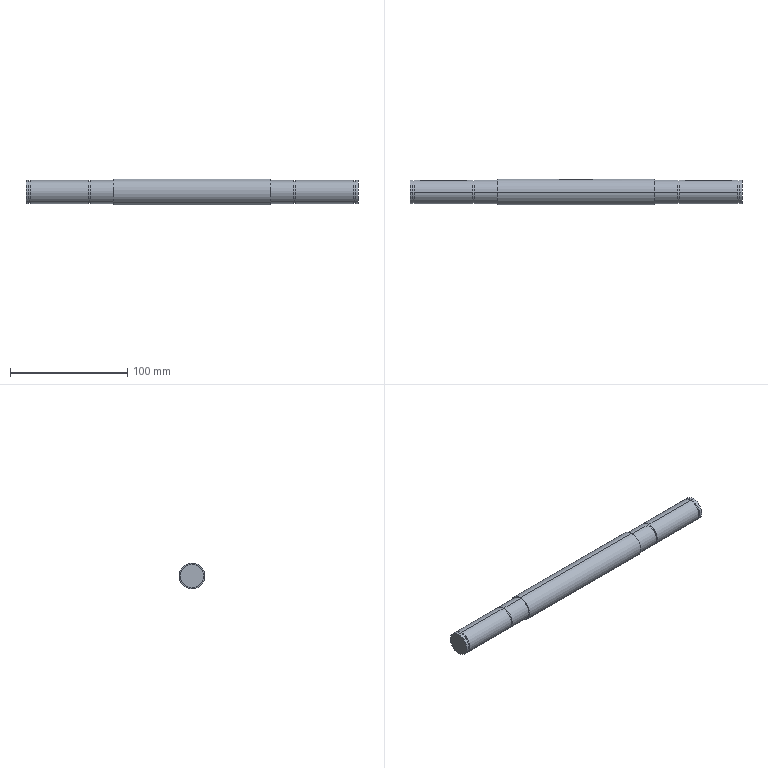Part | STEP file | Flat belt drive shaft | 1 solid | 49 faces | box 283.4 x 22 x 22 mm | volume 95567 mm3 | cylinder 28 | plane 21 | commonest cylinder face diameters 20 x12 19 x8 6 x6 22 x2
STEP:
#1=CARTESIAN_POINT('',(67.2,0.,-10.));
#2=VERTEX_POINT('',#1);
#3=CARTESIAN_POINT('',(67.2,0.,10.));
#4=VERTEX_POINT('',#3);
#5=CARTESIAN_POINT('',(67.2,0.,0.));
#6=DIRECTION('',(1.,0.,0.));
#7=DIRECTION('',(0.,0.,-1.));
#8=AXIS2_PLACEMENT_3D('',#5,#6,#7);
#9=CIRCLE('',#8,10.);
#10=EDGE_CURVE('',#2,#4,#9,.T.);
#11=ORIENTED_EDGE('',*,*,#10,.T.);
#12=CARTESIAN_POINT('',(87.,0.,10.));
#13=VERTEX_POINT('',#12);
#14=CARTESIAN_POINT('',(141.7,0.,10.));
#15=DIRECTION('',(1.,0.,0.));
#16=VECTOR('',#15,1000.);
#17=LINE('',#14,#16);
#18=EDGE_CURVE('',#4,#13,#17,.T.);
#19=ORIENTED_EDGE('',*,*,#18,.T.);
#20=CARTESIAN_POINT('',(87.,0.,-10.));
#21=VERTEX_POINT('',#20);
#22=CARTESIAN_POINT('',(87.,0.,0.));
#23=DIRECTION('',(1.,0.,0.));
#24=DIRECTION('',(0.,0.,-1.));
#25=AXIS2_PLACEMENT_3D('',#22,#23,#24);
#26=CIRCLE('',#25,10.);
#27=EDGE_CURVE('',#21,#13,#26,.T.);
#28=ORIENTED_EDGE('',*,*,#27,.F.);
#29=CARTESIAN_POINT('',(141.7,0.,-10.));
#30=DIRECTION('',(1.,0.,0.));
#31=VECTOR('',#30,1000.);
#32=LINE('',#29,#31);
#33=EDGE_CURVE('',#2,#21,#32,.T.);
#34=ORIENTED_EDGE('',*,*,#33,.F.);
#35=EDGE_LOOP('',(#11,#19,#28,#34));
#36=FACE_OUTER_BOUND('',#35,.T.);
#37=CARTESIAN_POINT('',(141.7,0.,0.));
#38=DIRECTION('',(1.,0.,0.));
#39=DIRECTION('',(0.,0.,-1.));
#40=AXIS2_PLACEMENT_3D('',#37,#38,#39);
#41=CYLINDRICAL_SURFACE('',#40,10.);
#42=ADVANCED_FACE('',(#36),#41,.T.);
#43=CARTESIAN_POINT('',(87.,0.,-9.5));
#44=VERTEX_POINT('',#43);
#45=CARTESIAN_POINT('',(87.,0.,9.5));
#46=VERTEX_POINT('',#45);
#47=CARTESIAN_POINT('',(87.,0.,0.));
#48=DIRECTION('',(1.,0.,0.));
#49=DIRECTION('',(0.,0.,-1.));
#50=AXIS2_PLACEMENT_3D('',#47,#48,#49);
#51=CIRCLE('',#50,9.5);
#52=EDGE_CURVE('',#44,#46,#51,.T.);
#53=ORIENTED_EDGE('',*,*,#52,.T.);
#54=CARTESIAN_POINT('',(88.1,0.,9.5));
#55=VERTEX_POINT('',#54);
#56=CARTESIAN_POINT('',(141.7,0.,9.5));
#57=DIRECTION('',(1.,0.,0.));
#58=VECTOR('',#57,1000.);
#59=LINE('',#56,#58);
#60=EDGE_CURVE('',#46,#55,#59,.T.);
#61=ORIENTED_EDGE('',*,*,#60,.T.);
#62=CARTESIAN_POINT('',(88.1,0.,-9.5));
#63=VERTEX_POINT('',#62);
#64=CARTESIAN_POINT('',(88.1,0.,0.));
#65=DIRECTION('',(1.,0.,0.));
#66=DIRECTION('',(0.,0.,-1.));
#67=AXIS2_PLACEMENT_3D('',#64,#65,#66);
#68=CIRCLE('',#67,9.5);
#69=EDGE_CURVE('',#63,#55,#68,.T.);
#70=ORIENTED_EDGE('',*,*,#69,.F.);
#71=CARTESIAN_POINT('',(141.7,0.,-9.5));
#72=DIRECTION('',(1.,0.,0.));
#73=VECTOR('',#72,1000.);
#74=LINE('',#71,#73);
#75=EDGE_CURVE('',#44,#63,#74,.T.);
#76=ORIENTED_EDGE('',*,*,#75,.F.);
#77=EDGE_LOOP('',(#53,#61,#70,#76));
#78=FACE_OUTER_BOUND('',#77,.T.);
#79=CARTESIAN_POINT('',(141.7,0.,0.));
#80=DIRECTION('',(1.,0.,0.));
#81=DIRECTION('',(0.,0.,-1.));
#82=AXIS2_PLACEMENT_3D('',#79,#80,#81);
#83=CYLINDRICAL_SURFACE('',#82,9.5);
#84=ADVANCED_FACE('',(#78),#83,.T.);
#85=CARTESIAN_POINT('',(130.6,9.539,3.));
#86=VERTEX_POINT('',#85);
#87=CARTESIAN_POINT('',(130.6,9.539,-3.));
#88=VERTEX_POINT('',#87);
#89=CARTESIAN_POINT('',(130.6,9.539,3.));
#90=CARTESIAN_POINT('',(130.799,9.539,3.));
#91=CARTESIAN_POINT('',(130.995,9.546,2.98));
#92=CARTESIAN_POINT('',(131.38,9.569,2.903));
#93=CARTESIAN_POINT('',(131.571,9.587,2.845));
#94=CARTESIAN_POINT('',(131.934,9.631,2.694));
#95=CARTESIAN_POINT('',(132.106,9.656,2.602));
#96=CARTESIAN_POINT('',(132.431,9.712,2.384));
#97=CARTESIAN_POINT('',(132.584,9.743,2.258));
#98=CARTESIAN_POINT('',(132.997,9.832,1.846));
#99=CARTESIAN_POINT('',(133.22,9.892,1.513));
#100=CARTESIAN_POINT('',(133.445,9.954,0.972));
#101=CARTESIAN_POINT('',(133.503,9.971,0.7816));
#102=CARTESIAN_POINT('',(133.581,9.994,0.3938));
#103=CARTESIAN_POINT('',(133.6,10.,0.1983));
#104=CARTESIAN_POINT('',(133.6,10.,-0.1957));
#105=CARTESIAN_POINT('',(133.58,9.994,-0.3958));
#106=CARTESIAN_POINT('',(133.503,9.971,-0.7816));
#107=CARTESIAN_POINT('',(133.446,9.955,-0.9692));
#108=CARTESIAN_POINT('',(133.294,9.912,-1.334));
#109=CARTESIAN_POINT('',(133.201,9.887,-1.508));
#110=CARTESIAN_POINT('',(132.984,9.832,-1.831));
#111=CARTESIAN_POINT('',(132.859,9.802,-1.984));
#112=CARTESIAN_POINT('',(132.582,9.742,-2.261));
#113=CARTESIAN_POINT('',(132.431,9.712,-2.384));
#114=CARTESIAN_POINT('',(132.107,9.656,-2.601));
#115=CARTESIAN_POINT('',(131.932,9.63,-2.695));
#116=CARTESIAN_POINT('',(131.57,9.587,-2.846));
#117=CARTESIAN_POINT('',(131.383,9.57,-2.903));
#118=CARTESIAN_POINT('',(130.996,9.546,-2.98));
#119=CARTESIAN_POINT('',(130.797,9.539,-3.));
#120=CARTESIAN_POINT('',(130.6,9.539,-3.));
#121=B_SPLINE_CURVE_WITH_KNOTS('',3,(#89,#90,#91,#92,#93,#94,#95,#96,#97,#98,#99,#100,#101,#102,#103,#104,#105,#106,#107,#108,#109,#110,#111,#112,#113,#114,#115,#116,#117,#118,#119,#120),.UNSPECIFIED.,.F.,.F.,(4,2,2,2,2,2,2,2,2,2,2,2,2,2,2,4),(0.,0.0005896,0.001179,0.001769,0.002358,0.003538,0.004127,0.004717,0.005307,0.005896,0.006486,0.007075,0.007665,0.008255,0.008844,0.009434),.UNSPECIFIED.);
#122=EDGE_CURVE('',#86,#88,#121,.T.);
#123=ORIENTED_EDGE('',*,*,#122,.F.);
#124=CARTESIAN_POINT('',(95.6,9.539,3.));
#125=VERTEX_POINT('',#124);
#126=CARTESIAN_POINT('',(141.7,9.539,3.));
#127=DIRECTION('',(1.,0.,0.));
#128=VECTOR('',#127,1000.);
#129=LINE('',#126,#128);
#130=EDGE_CURVE('',#125,#86,#129,.T.);
#131=ORIENTED_EDGE('',*,*,#130,.F.);
#132=CARTESIAN_POINT('',(95.6,9.539,-3.));
#133=VERTEX_POINT('',#132);
#134=CARTESIAN_POINT('',(95.6,9.539,-3.));
#135=CARTESIAN_POINT('',(95.404,9.539,-3.));
#136=CARTESIAN_POINT('',(95.207,9.546,-2.981));
#137=CARTESIAN_POINT('',(94.817,9.569,-2.903));
#138=CARTESIAN_POINT('',(94.63,9.587,-2.845));
#139=CARTESIAN_POINT('',(94.268,9.63,-2.695));
#140=CARTESIAN_POINT('',(94.092,9.656,-2.601));
#141=CARTESIAN_POINT('',(93.768,9.712,-2.384));
#142=CARTESIAN_POINT('',(93.618,9.742,-2.26));
#143=CARTESIAN_POINT('',(93.341,9.802,-1.984));
#144=CARTESIAN_POINT('',(93.216,9.832,-1.831));
#145=CARTESIAN_POINT('',(92.999,9.887,-1.508));
#146=CARTESIAN_POINT('',(92.906,9.912,-1.335));
#147=CARTESIAN_POINT('',(92.754,9.955,-0.9694));
#148=CARTESIAN_POINT('',(92.697,9.971,-0.7818));
#149=CARTESIAN_POINT('',(92.62,9.994,-0.3973));
#150=CARTESIAN_POINT('',(92.6,10.,-0.1979));
#151=CARTESIAN_POINT('',(92.6,10.,0.1975));
#152=CARTESIAN_POINT('',(92.619,9.994,0.393));
#153=CARTESIAN_POINT('',(92.696,9.971,0.7797));
#154=CARTESIAN_POINT('',(92.755,9.954,0.971));
#155=CARTESIAN_POINT('',(92.98,9.892,1.513));
#156=CARTESIAN_POINT('',(93.203,9.832,1.846));
#157=CARTESIAN_POINT('',(93.616,9.743,2.258));
#158=CARTESIAN_POINT('',(93.769,9.712,2.384));
#159=CARTESIAN_POINT('',(94.094,9.656,2.602));
#160=CARTESIAN_POINT('',(94.265,9.631,2.694));
#161=CARTESIAN_POINT('',(94.627,9.587,2.845));
#162=CARTESIAN_POINT('',(94.819,9.569,2.903));
#163=CARTESIAN_POINT('',(95.204,9.546,2.98));
#164=CARTESIAN_POINT('',(95.401,9.539,3.));
#165=CARTESIAN_POINT('',(95.6,9.539,3.));
#166=B_SPLINE_CURVE_WITH_KNOTS('',3,(#134,#135,#136,#137,#138,#139,#140,#141,#142,#143,#144,#145,#146,#147,#148,#149,#150,#151,#152,#153,#154,#155,#156,#157,#158,#159,#160,#161,#162,#163,#164,#165),.UNSPECIFIED.,.F.,.F.,(4,2,2,2,2,2,2,2,2,2,2,2,2,2,2,4),(0.009434,0.01002,0.01061,0.0112,0.01179,0.01238,0.01297,0.01356,0.01415,0.01474,0.01533,0.01651,0.0171,0.01769,0.01828,0.01887),.UNSPECIFIED.);
#167=EDGE_CURVE('',#133,#125,#166,.T.);
#168=ORIENTED_EDGE('',*,*,#167,.F.);
#169=CARTESIAN_POINT('',(141.7,9.539,-3.));
#170=DIRECTION('',(-1.,0.,0.));
#171=VECTOR('',#170,1000.);
#172=LINE('',#169,#171);
#173=EDGE_CURVE('',#88,#133,#172,.T.);
#174=ORIENTED_EDGE('',*,*,#173,.F.);
#175=EDGE_LOOP('',(#123,#131,#168,#174));
#176=FACE_BOUND('',#175,.T.);
#177=CARTESIAN_POINT('',(88.1,0.,-10.));
#178=VERTEX_POINT('',#177);
#179=CARTESIAN_POINT('',(88.1,0.,10.));
#180=VERTEX_POINT('',#179);
#181=CARTESIAN_POINT('',(88.1,0.,0.));
#182=DIRECTION('',(1.,0.,0.));
#183=DIRECTION('',(0.,0.,-1.));
#184=AXIS2_PLACEMENT_3D('',#181,#182,#183);
#185=CIRCLE('',#184,10.);
#186=EDGE_CURVE('',#178,#180,#185,.T.);
#187=ORIENTED_EDGE('',*,*,#186,.T.);
#188=CARTESIAN_POINT('',(138.1,0.,10.));
#189=VERTEX_POINT('',#188);
#190=CARTESIAN_POINT('',(141.7,0.,10.));
#191=DIRECTION('',(1.,0.,0.));
#192=VECTOR('',#191,1000.);
#193=LINE('',#190,#192);
#194=EDGE_CURVE('',#180,#189,#193,.T.);
#195=ORIENTED_EDGE('',*,*,#194,.T.);
#196=CARTESIAN_POINT('',(138.1,0.,-10.));
#197=VERTEX_POINT('',#196);
#198=CARTESIAN_POINT('',(138.1,0.,0.));
#199=DIRECTION('',(1.,0.,0.));
#200=DIRECTION('',(0.,0.,-1.));
#201=AXIS2_PLACEMENT_3D('',#198,#199,#200);
#202=CIRCLE('',#201,10.);
#203=EDGE_CURVE('',#197,#189,#202,.T.);
#204=ORIENTED_EDGE('',*,*,#203,.F.);
#205=CARTESIAN_POINT('',(141.7,0.,-10.));
#206=DIRECTION('',(1.,0.,0.));
#207=VECTOR('',#206,1000.);
#208=LINE('',#205,#207);
#209=EDGE_CURVE('',#178,#197,#208,.T.);
#210=ORIENTED_EDGE('',*,*,#209,.F.);
#211=EDGE_LOOP('',(#187,#195,#204,#210));
#212=FACE_OUTER_BOUND('',#211,.T.);
#213=CARTESIAN_POINT('',(141.7,0.,0.));
#214=DIRECTION('',(1.,0.,0.));
#215=DIRECTION('',(0.,0.,-1.));
#216=AXIS2_PLACEMENT_3D('',#213,#214,#215);
#217=CYLINDRICAL_SURFACE('',#216,10.);
#218=ADVANCED_FACE('',(#176,#212),#217,.T.);
#219=CARTESIAN_POINT('',(138.1,0.,-9.5));
#220=VERTEX_POINT('',#219);
#221=CARTESIAN_POINT('',(138.1,0.,9.5));
#222=VERTEX_POINT('',#221);
#223=CARTESIAN_POINT('',(138.1,0.,0.));
#224=DIRECTION('',(1.,0.,0.));
#225=DIRECTION('',(0.,0.,-1.));
#226=AXIS2_PLACEMENT_3D('',#223,#224,#225);
#227=CIRCLE('',#226,9.5);
#228=EDGE_CURVE('',#220,#222,#227,.T.);
#229=ORIENTED_EDGE('',*,*,#228,.T.);
#230=CARTESIAN_POINT('',(139.2,0.,9.5));
#231=VERTEX_POINT('',#230);
#232=CARTESIAN_POINT('',(141.7,0.,9.5));
#233=DIRECTION('',(1.,0.,0.));
#234=VECTOR('',#233,1000.);
#235=LINE('',#232,#234);
#236=EDGE_CURVE('',#222,#231,#235,.T.);
#237=ORIENTED_EDGE('',*,*,#236,.T.);
#238=CARTESIAN_POINT('',(139.2,0.,-9.5));
#239=VERTEX_POINT('',#238);
#240=CARTESIAN_POINT('',(139.2,0.,0.));
#241=DIRECTION('',(1.,0.,0.));
#242=DIRECTION('',(0.,0.,-1.));
#243=AXIS2_PLACEMENT_3D('',#240,#241,#242);
#244=CIRCLE('',#243,9.5);
#245=EDGE_CURVE('',#239,#231,#244,.T.);
#246=ORIENTED_EDGE('',*,*,#245,.F.);
#247=CARTESIAN_POINT('',(141.7,0.,-9.5));
#248=DIRECTION('',(1.,0.,0.));
#249=VECTOR('',#248,1000.);
#250=LINE('',#247,#249);
#251=EDGE_CURVE('',#220,#239,#250,.T.);
#252=ORIENTED_EDGE('',*,*,#251,.F.);
#253=EDGE_LOOP('',(#229,#237,#246,#252));
#254=FACE_OUTER_BOUND('',#253,.T.);
#255=CARTESIAN_POINT('',(141.7,0.,0.));
#256=DIRECTION('',(1.,0.,0.));
#257=DIRECTION('',(0.,0.,-1.));
#258=AXIS2_PLACEMENT_3D('',#255,#256,#257);
#259=CYLINDRICAL_SURFACE('',#258,9.5);
#260=ADVANCED_FACE('',(#254),#259,.T.);
#261=CARTESIAN_POINT('',(139.2,0.,-10.));
#262=VERTEX_POINT('',#261);
#263=CARTESIAN_POINT('',(139.2,0.,10.));
#264=VERTEX_POINT('',#263);
#265=CARTESIAN_POINT('',(139.2,0.,0.));
#266=DIRECTION('',(1.,0.,0.));
#267=DIRECTION('',(0.,0.,-1.));
#268=AXIS2_PLACEMENT_3D('',#265,#266,#267);
#269=CIRCLE('',#268,10.);
#270=EDGE_CURVE('',#262,#264,#269,.T.);
#271=ORIENTED_EDGE('',*,*,#270,.T.);
#272=CARTESIAN_POINT('',(141.7,0.,10.));
#273=VERTEX_POINT('',#272);
#274=CARTESIAN_POINT('',(141.7,0.,10.));
#275=DIRECTION('',(1.,0.,0.));
#276=VECTOR('',#275,1000.);
#277=LINE('',#274,#276);
#278=EDGE_CURVE('',#264,#273,#277,.T.);
#279=ORIENTED_EDGE('',*,*,#278,.T.);
#280=CARTESIAN_POINT('',(141.7,0.,-10.));
#281=VERTEX_POINT('',#280);
#282=CARTESIAN_POINT('',(141.7,0.,0.));
#283=DIRECTION('',(1.,0.,0.));
#284=DIRECTION('',(0.,0.,-1.));
#285=AXIS2_PLACEMENT_3D('',#282,#283,#284);
#286=CIRCLE('',#285,10.);
#287=EDGE_CURVE('',#281,#273,#286,.T.);
#288=ORIENTED_EDGE('',*,*,#287,.F.);
#289=CARTESIAN_POINT('',(141.7,0.,-10.));
#290=DIRECTION('',(1.,0.,0.));
#291=VECTOR('',#290,1000.);
#292=LINE('',#289,#291);
#293=EDGE_CURVE('',#262,#281,#292,.T.);
#294=ORIENTED_EDGE('',*,*,#293,.F.);
#295=EDGE_LOOP('',(#271,#279,#288,#294));
#296=FACE_OUTER_BOUND('',#295,.T.);
#297=CARTESIAN_POINT('',(141.7,0.,0.));
#298=DIRECTION('',(1.,0.,0.));
#299=DIRECTION('',(0.,0.,-1.));
#300=AXIS2_PLACEMENT_3D('',#297,#298,#299);
#301=CYLINDRICAL_SURFACE('',#300,10.);
#302=ADVANCED_FACE('',(#296),#301,.T.);
#303=CARTESIAN_POINT('',(-141.7,0.,-10.));
#304=VERTEX_POINT('',#303);
#305=CARTESIAN_POINT('',(-141.7,0.,10.));
#306=VERTEX_POINT('',#305);
#307=CARTESIAN_POINT('',(-141.7,0.,0.));
#308=DIRECTION('',(1.,0.,0.));
#309=DIRECTION('',(0.,0.,-1.));
#310=AXIS2_PLACEMENT_3D('',#307,#308,#309);
#311=CIRCLE('',#310,10.);
#312=EDGE_CURVE('',#304,#306,#311,.T.);
#313=ORIENTED_EDGE('',*,*,#312,.T.);
#314=CARTESIAN_POINT('',(-139.2,0.,10.));
#315=VERTEX_POINT('',#314);
#316=CARTESIAN_POINT('',(141.7,0.,10.));
#317=DIRECTION('',(1.,0.,0.));
#318=VECTOR('',#317,1000.);
#319=LINE('',#316,#318);
#320=EDGE_CURVE('',#306,#315,#319,.T.);
#321=ORIENTED_EDGE('',*,*,#320,.T.);
#322=CARTESIAN_POINT('',(-139.2,0.,-10.));
#323=VERTEX_POINT('',#322);
#324=CARTESIAN_POINT('',(-139.2,0.,0.));
#325=DIRECTION('',(1.,0.,0.));
#326=DIRECTION('',(0.,0.,-1.));
#327=AXIS2_PLACEMENT_3D('',#324,#325,#326);
#328=CIRCLE('',#327,10.);
#329=EDGE_CURVE('',#323,#315,#328,.T.);
#330=ORIENTED_EDGE('',*,*,#329,.F.);
#331=CARTESIAN_POINT('',(141.7,0.,-10.));
#332=DIRECTION('',(1.,0.,0.));
#333=VECTOR('',#332,1000.);
#334=LINE('',#331,#333);
#335=EDGE_CURVE('',#304,#323,#334,.T.);
#336=ORIENTED_EDGE('',*,*,#335,.F.);
#337=EDGE_LOOP('',(#313,#321,#330,#336));
#338=FACE_OUTER_BOUND('',#337,.T.);
#339=CARTESIAN_POINT('',(141.7,0.,0.));
#340=DIRECTION('',(1.,0.,0.));
#341=DIRECTION('',(0.,0.,-1.));
#342=AXIS2_PLACEMENT_3D('',#339,#340,#341);
#343=CYLINDRICAL_SURFACE('',#342,10.);
#344=ADVANCED_FACE('',(#338),#343,.T.);
#345=CARTESIAN_POINT('',(-139.2,0.,-9.5));
#346=VERTEX_POINT('',#345);
#347=CARTESIAN_POINT('',(-139.2,0.,9.5));
#348=VERTEX_POINT('',#347);
#349=CARTESIAN_POINT('',(-139.2,0.,0.));
#350=DIRECTION('',(1.,0.,0.));
#351=DIRECTION('',(0.,0.,-1.));
#352=AXIS2_PLACEMENT_3D('',#349,#350,#351);
#353=CIRCLE('',#352,9.5);
#354=EDGE_CURVE('',#346,#348,#353,.T.);
#355=ORIENTED_EDGE('',*,*,#354,.T.);
#356=CARTESIAN_POINT('',(-138.1,0.,9.5));
#357=VERTEX_POINT('',#356);
#358=CARTESIAN_POINT('',(141.7,0.,9.5));
#359=DIRECTION('',(1.,0.,0.));
#360=VECTOR('',#359,1000.);
#361=LINE('',#358,#360);
#362=EDGE_CURVE('',#348,#357,#361,.T.);
#363=ORIENTED_EDGE('',*,*,#362,.T.);
#364=CARTESIAN_POINT('',(-138.1,0.,-9.5));
#365=VERTEX_POINT('',#364);
#366=CARTESIAN_POINT('',(-138.1,0.,0.));
#367=DIRECTION('',(1.,0.,0.));
#368=DIRECTION('',(0.,0.,-1.));
#369=AXIS2_PLACEMENT_3D('',#366,#367,#368);
#370=CIRCLE('',#369,9.5);
#371=EDGE_CURVE('',#365,#357,#370,.T.);
#372=ORIENTED_EDGE('',*,*,#371,.F.);
#373=CARTESIAN_POINT('',(141.7,0.,-9.5));
#374=DIRECTION('',(1.,0.,0.));
#375=VECTOR('',#374,1000.);
#376=LINE('',#373,#375);
#377=EDGE_CURVE('',#346,#365,#376,.T.);
#378=ORIENTED_EDGE('',*,*,#377,.F.);
#379=EDGE_LOOP('',(#355,#363,#372,#378));
#380=FACE_OUTER_BOUND('',#379,.T.);
#381=CARTESIAN_POINT('',(141.7,0.,0.));
#382=DIRECTION('',(1.,0.,0.));
#383=DIRECTION('',(0.,0.,-1.));
#384=AXIS2_PLACEMENT_3D('',#381,#382,#383);
#385=CYLINDRICAL_SURFACE('',#384,9.5);
#386=ADVANCED_FACE('',(#380),#385,.T.);
#387=CARTESIAN_POINT('',(-130.6,9.539,-3.));
#388=VERTEX_POINT('',#387);
#389=CARTESIAN_POINT('',(-130.6,9.539,3.));
#390=VERTEX_POINT('',#389);
#391=CARTESIAN_POINT('',(-130.6,9.539,-3.));
#392=CARTESIAN_POINT('',(-130.796,9.539,-3.));
#393=CARTESIAN_POINT('',(-130.993,9.546,-2.981));
#394=CARTESIAN_POINT('',(-131.383,9.569,-2.903));
#395=CARTESIAN_POINT('',(-131.57,9.587,-2.845));
#396=CARTESIAN_POINT('',(-131.932,9.63,-2.695));
#397=CARTESIAN_POINT('',(-132.108,9.656,-2.601));
#398=CARTESIAN_POINT('',(-132.432,9.712,-2.384));
#399=CARTESIAN_POINT('',(-132.582,9.742,-2.26));
#400=CARTESIAN_POINT('',(-132.859,9.802,-1.984));
#401=CARTESIAN_POINT('',(-132.984,9.832,-1.831));
#402=CARTESIAN_POINT('',(-133.201,9.887,-1.508));
#403=CARTESIAN_POINT('',(-133.294,9.912,-1.335));
#404=CARTESIAN_POINT('',(-133.446,9.955,-0.9694));
#405=CARTESIAN_POINT('',(-133.503,9.971,-0.7818));
#406=CARTESIAN_POINT('',(-133.58,9.994,-0.3973));
#407=CARTESIAN_POINT('',(-133.6,10.,-0.1979));
#408=CARTESIAN_POINT('',(-133.6,10.,0.1975));
#409=CARTESIAN_POINT('',(-133.581,9.994,0.393));
#410=CARTESIAN_POINT('',(-133.504,9.971,0.7797));
#411=CARTESIAN_POINT('',(-133.445,9.954,0.971));
#412=CARTESIAN_POINT('',(-133.22,9.892,1.513));
#413=CARTESIAN_POINT('',(-132.997,9.832,1.846));
#414=CARTESIAN_POINT('',(-132.584,9.743,2.258));
#415=CARTESIAN_POINT('',(-132.431,9.712,2.384));
#416=CARTESIAN_POINT('',(-132.106,9.656,2.602));
#417=CARTESIAN_POINT('',(-131.935,9.631,2.694));
#418=CARTESIAN_POINT('',(-131.573,9.587,2.845));
#419=CARTESIAN_POINT('',(-131.381,9.569,2.903));
#420=CARTESIAN_POINT('',(-130.996,9.546,2.98));
#421=CARTESIAN_POINT('',(-130.799,9.539,3.));
#422=CARTESIAN_POINT('',(-130.6,9.539,3.));
#423=B_SPLINE_CURVE_WITH_KNOTS('',3,(#391,#392,#393,#394,#395,#396,#397,#398,#399,#400,#401,#402,#403,#404,#405,#406,#407,#408,#409,#410,#411,#412,#413,#414,#415,#416,#417,#418,#419,#420,#421,#422),.UNSPECIFIED.,.F.,.F.,(4,2,2,2,2,2,2,2,2,2,2,2,2,2,2,4),(0.009434,0.01002,0.01061,0.0112,0.01179,0.01238,0.01297,0.01356,0.01415,0.01474,0.01533,0.01651,0.0171,0.01769,0.01828,0.01887),.UNSPECIFIED.);
#424=EDGE_CURVE('',#388,#390,#423,.T.);
#425=ORIENTED_EDGE('',*,*,#424,.F.);
#426=CARTESIAN_POINT('',(-95.6,9.539,-3.));
#427=VERTEX_POINT('',#426);
#428=CARTESIAN_POINT('',(141.7,9.539,-3.));
#429=DIRECTION('',(-1.,0.,0.));
#430=VECTOR('',#429,1000.);
#431=LINE('',#428,#430);
#432=EDGE_CURVE('',#427,#388,#431,.T.);
#433=ORIENTED_EDGE('',*,*,#432,.F.);
#434=CARTESIAN_POINT('',(-95.6,9.539,3.));
#435=VERTEX_POINT('',#434);
#436=CARTESIAN_POINT('',(-95.6,9.539,3.));
#437=CARTESIAN_POINT('',(-95.401,9.539,3.));
#438=CARTESIAN_POINT('',(-95.205,9.546,2.98));
#439=CARTESIAN_POINT('',(-94.82,9.569,2.903));
#440=CARTESIAN_POINT('',(-94.629,9.587,2.845));
#441=CARTESIAN_POINT('',(-94.266,9.631,2.694));
#442=CARTESIAN_POINT('',(-94.094,9.656,2.602));
#443=CARTESIAN_POINT('',(-93.769,9.712,2.384));
#444=CARTESIAN_POINT('',(-93.616,9.743,2.258));
#445=CARTESIAN_POINT('',(-93.203,9.832,1.846));
#446=CARTESIAN_POINT('',(-92.98,9.892,1.513));
#447=CARTESIAN_POINT('',(-92.755,9.954,0.972));
#448=CARTESIAN_POINT('',(-92.697,9.971,0.7816));
#449=CARTESIAN_POINT('',(-92.619,9.994,0.3938));
#450=CARTESIAN_POINT('',(-92.6,10.,0.1983));
#451=CARTESIAN_POINT('',(-92.6,10.,-0.1957));
#452=CARTESIAN_POINT('',(-92.62,9.994,-0.3958));
#453=CARTESIAN_POINT('',(-92.697,9.971,-0.7816));
#454=CARTESIAN_POINT('',(-92.754,9.955,-0.9692));
#455=CARTESIAN_POINT('',(-92.906,9.912,-1.334));
#456=CARTESIAN_POINT('',(-92.999,9.887,-1.508));
#457=CARTESIAN_POINT('',(-93.216,9.832,-1.831));
#458=CARTESIAN_POINT('',(-93.341,9.802,-1.984));
#459=CARTESIAN_POINT('',(-93.618,9.742,-2.261));
#460=CARTESIAN_POINT('',(-93.769,9.712,-2.384));
#461=CARTESIAN_POINT('',(-94.093,9.656,-2.601));
#462=CARTESIAN_POINT('',(-94.268,9.63,-2.695));
#463=CARTESIAN_POINT('',(-94.63,9.587,-2.846));
#464=CARTESIAN_POINT('',(-94.817,9.57,-2.903));
#465=CARTESIAN_POINT('',(-95.204,9.546,-2.98));
#466=CARTESIAN_POINT('',(-95.403,9.539,-3.));
#467=CARTESIAN_POINT('',(-95.6,9.539,-3.));
#468=B_SPLINE_CURVE_WITH_KNOTS('',3,(#436,#437,#438,#439,#440,#441,#442,#443,#444,#445,#446,#447,#448,#449,#450,#451,#452,#453,#454,#455,#456,#457,#458,#459,#460,#461,#462,#463,#464,#465,#466,#467),.UNSPECIFIED.,.F.,.F.,(4,2,2,2,2,2,2,2,2,2,2,2,2,2,2,4),(0.,0.0005896,0.001179,0.001769,0.002358,0.003538,0.004127,0.004717,0.005307,0.005896,0.006486,0.007075,0.007665,0.008255,0.008844,0.009434),.UNSPECIFIED.);
#469=EDGE_CURVE('',#435,#427,#468,.T.);
#470=ORIENTED_EDGE('',*,*,#469,.F.);
#471=CARTESIAN_POINT('',(141.7,9.539,3.));
#472=DIRECTION('',(1.,0.,0.));
#473=VECTOR('',#472,1000.);
#474=LINE('',#471,#473);
#475=EDGE_CURVE('',#390,#435,#474,.T.);
#476=ORIENTED_EDGE('',*,*,#475,.F.);
#477=EDGE_LOOP('',(#425,#433,#470,#476));
#478=FACE_BOUND('',#477,.T.);
#479=CARTESIAN_POINT('',(-138.1,0.,-10.));
#480=VERTEX_POINT('',#479);
#481=CARTESIAN_POINT('',(-138.1,0.,10.));
#482=VERTEX_POINT('',#481);
#483=CARTESIAN_POINT('',(-138.1,0.,0.));
#484=DIRECTION('',(1.,0.,0.));
#485=DIRECTION('',(0.,0.,-1.));
#486=AXIS2_PLACEMENT_3D('',#483,#484,#485);
#487=CIRCLE('',#486,10.);
#488=EDGE_CURVE('',#480,#482,#487,.T.);
#489=ORIENTED_EDGE('',*,*,#488,.T.);
#490=CARTESIAN_POINT('',(-88.1,0.,10.));
#491=VERTEX_POINT('',#490);
#492=CARTESIAN_POINT('',(141.7,0.,10.));
#493=DIRECTION('',(1.,0.,0.));
#494=VECTOR('',#493,1000.);
#495=LINE('',#492,#494);
#496=EDGE_CURVE('',#482,#491,#495,.T.);
#497=ORIENTED_EDGE('',*,*,#496,.T.);
#498=CARTESIAN_POINT('',(-88.1,0.,-10.));
#499=VERTEX_POINT('',#498);
#500=CARTESIAN_POINT('',(-88.1,0.,0.));
#501=DIRECTION('',(1.,0.,0.));
#502=DIRECTION('',(0.,0.,-1.));
#503=AXIS2_PLACEMENT_3D('',#500,#501,#502);
#504=CIRCLE('',#503,10.);
#505=EDGE_CURVE('',#499,#491,#504,.T.);
#506=ORIENTED_EDGE('',*,*,#505,.F.);
#507=CARTESIAN_POINT('',(141.7,0.,-10.));
#508=DIRECTION('',(1.,0.,0.));
#509=VECTOR('',#508,1000.);
#510=LINE('',#507,#509);
#511=EDGE_CURVE('',#480,#499,#510,.T.);
#512=ORIENTED_EDGE('',*,*,#511,.F.);
#513=EDGE_LOOP('',(#489,#497,#506,#512));
#514=FACE_OUTER_BOUND('',#513,.T.);
#515=CARTESIAN_POINT('',(141.7,0.,0.));
#516=DIRECTION('',(1.,0.,0.));
#517=DIRECTION('',(0.,0.,-1.));
#518=AXIS2_PLACEMENT_3D('',#515,#516,#517);
#519=CYLINDRICAL_SURFACE('',#518,10.);
#520=ADVANCED_FACE('',(#478,#514),#519,.T.);
#521=CARTESIAN_POINT('',(-88.1,0.,-9.5));
#522=VERTEX_POINT('',#521);
#523=CARTESIAN_POINT('',(-88.1,0.,9.5));
#524=VERTEX_POINT('',#523);
#525=CARTESIAN_POINT('',(-88.1,0.,0.));
#526=DIRECTION('',(1.,0.,0.));
#527=DIRECTION('',(0.,0.,-1.));
#528=AXIS2_PLACEMENT_3D('',#525,#526,#527);
#529=CIRCLE('',#528,9.5);
#530=EDGE_CURVE('',#522,#524,#529,.T.);
#531=ORIENTED_EDGE('',*,*,#530,.T.);
#532=CARTESIAN_POINT('',(-87.,0.,9.5));
#533=VERTEX_POINT('',#532);
#534=CARTESIAN_POINT('',(141.7,0.,9.5));
#535=DIRECTION('',(1.,0.,0.));
#536=VECTOR('',#535,1000.);
#537=LINE('',#534,#536);
#538=EDGE_CURVE('',#524,#533,#537,.T.);
#539=ORIENTED_EDGE('',*,*,#538,.T.);
#540=CARTESIAN_POINT('',(-87.,0.,-9.5));
#541=VERTEX_POINT('',#540);
#542=CARTESIAN_POINT('',(-87.,0.,0.));
#543=DIRECTION('',(1.,0.,0.));
#544=DIRECTION('',(0.,0.,-1.));
#545=AXIS2_PLACEMENT_3D('',#542,#543,#544);
#546=CIRCLE('',#545,9.5);
#547=EDGE_CURVE('',#541,#533,#546,.T.);
#548=ORIENTED_EDGE('',*,*,#547,.F.);
#549=CARTESIAN_POINT('',(141.7,0.,-9.5));
#550=DIRECTION('',(1.,0.,0.));
#551=VECTOR('',#550,1000.);
#552=LINE('',#549,#551);
#553=EDGE_CURVE('',#522,#541,#552,.T.);
#554=ORIENTED_EDGE('',*,*,#553,.F.);
#555=EDGE_LOOP('',(#531,#539,#548,#554));
#556=FACE_OUTER_BOUND('',#555,.T.);
#557=CARTESIAN_POINT('',(141.7,0.,0.));
#558=DIRECTION('',(1.,0.,0.));
#559=DIRECTION('',(0.,0.,-1.));
#560=AXIS2_PLACEMENT_3D('',#557,#558,#559);
#561=CYLINDRICAL_SURFACE('',#560,9.5);
#562=ADVANCED_FACE('',(#556),#561,.T.);
#563=CARTESIAN_POINT('',(-87.,0.,-10.));
#564=VERTEX_POINT('',#563);
#565=CARTESIAN_POINT('',(-87.,0.,10.));
#566=VERTEX_POINT('',#565);
#567=CARTESIAN_POINT('',(-87.,0.,0.));
#568=DIRECTION('',(1.,0.,0.));
#569=DIRECTION('',(0.,0.,-1.));
#570=AXIS2_PLACEMENT_3D('',#567,#568,#569);
#571=CIRCLE('',#570,10.);
#572=EDGE_CURVE('',#564,#566,#571,.T.);
#573=ORIENTED_EDGE('',*,*,#572,.T.);
#574=CARTESIAN_POINT('',(-67.2,0.,10.));
#575=VERTEX_POINT('',#574);
#576=CARTESIAN_POINT('',(141.7,0.,10.));
#577=DIRECTION('',(1.,0.,0.));
#578=VECTOR('',#577,1000.);
#579=LINE('',#576,#578);
#580=EDGE_CURVE('',#566,#575,#579,.T.);
#581=ORIENTED_EDGE('',*,*,#580,.T.);
#582=CARTESIAN_POINT('',(-67.2,0.,-10.));
#583=VERTEX_POINT('',#582);
#584=CARTESIAN_POINT('',(-67.2,0.,0.));
#585=DIRECTION('',(1.,0.,0.));
#586=DIRECTION('',(0.,0.,-1.));
#587=AXIS2_PLACEMENT_3D('',#584,#585,#586);
#588=CIRCLE('',#587,10.);
#589=EDGE_CURVE('',#583,#575,#588,.T.);
#590=ORIENTED_EDGE('',*,*,#589,.F.);
#591=CARTESIAN_POINT('',(141.7,0.,-10.));
#592=DIRECTION('',(1.,0.,0.));
#593=VECTOR('',#592,1000.);
#594=LINE('',#591,#593);
#595=EDGE_CURVE('',#564,#583,#594,.T.);
#596=ORIENTED_EDGE('',*,*,#595,.F.);
#597=EDGE_LOOP('',(#573,#581,#590,#596));
#598=FACE_OUTER_BOUND('',#597,.T.);
#599=CARTESIAN_POINT('',(141.7,0.,0.));
#600=DIRECTION('',(1.,0.,0.));
#601=DIRECTION('',(0.,0.,-1.));
#602=AXIS2_PLACEMENT_3D('',#599,#600,#601);
#603=CYLINDRICAL_SURFACE('',#602,10.);
#604=ADVANCED_FACE('',(#598),#603,.T.);
#605=CARTESIAN_POINT('',(12.5,10.583,3.));
#606=VERTEX_POINT('',#605);
#607=CARTESIAN_POINT('',(12.5,10.583,-3.));
#608=VERTEX_POINT('',#607);
#609=CARTESIAN_POINT('',(12.5,10.583,3.));
#610=CARTESIAN_POINT('',(12.699,10.583,3.));
#611=CARTESIAN_POINT('',(12.895,10.589,2.98));
#612=CARTESIAN_POINT('',(13.279,10.61,2.904));
#613=CARTESIAN_POINT('',(13.47,10.626,2.846));
#614=CARTESIAN_POINT('',(13.833,10.665,2.695));
#615=CARTESIAN_POINT('',(14.005,10.688,2.603));
#616=CARTESIAN_POINT('',(14.33,10.739,2.385));
#617=CARTESIAN_POINT('',(14.484,10.766,2.259));
#618=CARTESIAN_POINT('',(14.759,10.821,1.984));
#619=CARTESIAN_POINT('',(14.883,10.847,1.833));
#620=CARTESIAN_POINT('',(15.102,10.898,1.506));
#621=CARTESIAN_POINT('',(15.195,10.92,1.333));
#622=CARTESIAN_POINT('',(15.345,10.958,0.9724));
#623=CARTESIAN_POINT('',(15.403,10.974,0.7823));
#624=CARTESIAN_POINT('',(15.48,10.995,0.3947));
#625=CARTESIAN_POINT('',(15.5,11.,0.1995));
#626=CARTESIAN_POINT('',(15.5,11.,-0.1939));
#627=CARTESIAN_POINT('',(15.481,10.995,-0.3937));
#628=CARTESIAN_POINT('',(15.404,10.974,-0.7792));
#629=CARTESIAN_POINT('',(15.347,10.959,-0.9667));
#630=CARTESIAN_POINT('',(15.12,10.902,-1.513));
#631=CARTESIAN_POINT('',(14.899,10.848,-1.843));
#632=CARTESIAN_POINT('',(14.483,10.766,-2.259));
#633=CARTESIAN_POINT('',(14.333,10.739,-2.383));
#634=CARTESIAN_POINT('',(14.009,10.689,-2.6));
#635=CARTESIAN_POINT('',(13.834,10.665,-2.694));
#636=CARTESIAN_POINT('',(13.472,10.626,-2.845));
#637=CARTESIAN_POINT('',(13.285,10.61,-2.902));
#638=CARTESIAN_POINT('',(12.898,10.589,-2.98));
#639=CARTESIAN_POINT('',(12.699,10.583,-3.));
#640=CARTESIAN_POINT('',(12.5,10.583,-3.));
#641=B_SPLINE_CURVE_WITH_KNOTS('',3,(#609,#610,#611,#612,#613,#614,#615,#616,#617,#618,#619,#620,#621,#622,#623,#624,#625,#626,#627,#628,#629,#630,#631,#632,#633,#634,#635,#636,#637,#638,#639,#640),.UNSPECIFIED.,.F.,.F.,(4,2,2,2,2,2,2,2,2,2,2,2,2,2,2,4),(0.,0.0005888,0.001178,0.001766,0.002355,0.002944,0.003533,0.004122,0.004711,0.005299,0.005888,0.007066,0.007655,0.008243,0.008832,0.009421),.UNSPECIFIED.);
#642=EDGE_CURVE('',#606,#608,#641,.T.);
#643=ORIENTED_EDGE('',*,*,#642,.F.);
#644=CARTESIAN_POINT('',(-12.5,10.583,3.));
#645=VERTEX_POINT('',#644);
#646=CARTESIAN_POINT('',(141.7,10.583,3.));
#647=DIRECTION('',(1.,0.,0.));
#648=VECTOR('',#647,1000.);
#649=LINE('',#646,#648);
#650=EDGE_CURVE('',#645,#606,#649,.T.);
#651=ORIENTED_EDGE('',*,*,#650,.F.);
#652=CARTESIAN_POINT('',(-12.5,10.583,-3.));
#653=VERTEX_POINT('',#652);
#654=CARTESIAN_POINT('',(-12.5,10.583,-3.));
#655=CARTESIAN_POINT('',(-12.699,10.583,-3.));
#656=CARTESIAN_POINT('',(-12.895,10.589,-2.98));
#657=CARTESIAN_POINT('',(-13.279,10.61,-2.904));
#658=CARTESIAN_POINT('',(-13.47,10.626,-2.846));
#659=CARTESIAN_POINT('',(-13.833,10.665,-2.695));
#660=CARTESIAN_POINT('',(-14.005,10.688,-2.603));
#661=CARTESIAN_POINT('',(-14.33,10.739,-2.385));
#662=CARTESIAN_POINT('',(-14.484,10.766,-2.259));
#663=CARTESIAN_POINT('',(-14.759,10.821,-1.984));
#664=CARTESIAN_POINT('',(-14.883,10.847,-1.833));
#665=CARTESIAN_POINT('',(-15.102,10.898,-1.506));
#666=CARTESIAN_POINT('',(-15.195,10.92,-1.333));
#667=CARTESIAN_POINT('',(-15.345,10.958,-0.9724));
#668=CARTESIAN_POINT('',(-15.403,10.974,-0.7823));
#669=CARTESIAN_POINT('',(-15.48,10.995,-0.3947));
#670=CARTESIAN_POINT('',(-15.5,11.,-0.1995));
#671=CARTESIAN_POINT('',(-15.5,11.,0.1939));
#672=CARTESIAN_POINT('',(-15.481,10.995,0.3937));
#673=CARTESIAN_POINT('',(-15.404,10.974,0.7792));
#674=CARTESIAN_POINT('',(-15.347,10.959,0.9667));
#675=CARTESIAN_POINT('',(-15.12,10.902,1.513));
#676=CARTESIAN_POINT('',(-14.899,10.848,1.843));
#677=CARTESIAN_POINT('',(-14.483,10.766,2.259));
#678=CARTESIAN_POINT('',(-14.333,10.739,2.383));
#679=CARTESIAN_POINT('',(-14.009,10.689,2.6));
#680=CARTESIAN_POINT('',(-13.834,10.665,2.694));
#681=CARTESIAN_POINT('',(-13.472,10.626,2.845));
#682=CARTESIAN_POINT('',(-13.285,10.61,2.902));
#683=CARTESIAN_POINT('',(-12.898,10.589,2.98));
#684=CARTESIAN_POINT('',(-12.699,10.583,3.));
#685=CARTESIAN_POINT('',(-12.5,10.583,3.));
#686=B_SPLINE_CURVE_WITH_KNOTS('',3,(#654,#655,#656,#657,#658,#659,#660,#661,#662,#663,#664,#665,#666,#667,#668,#669,#670,#671,#672,#673,#674,#675,#676,#677,#678,#679,#680,#681,#682,#683,#684,#685),.UNSPECIFIED.,.F.,.F.,(4,2,2,2,2,2,2,2,2,2,2,2,2,2,2,4),(0.,0.0005888,0.001178,0.001766,0.002355,0.002944,0.003533,0.004122,0.004711,0.005299,0.005888,0.007066,0.007655,0.008243,0.008832,0.009421),.UNSPECIFIED.);
#687=EDGE_CURVE('',#653,#645,#686,.T.);
#688=ORIENTED_EDGE('',*,*,#687,.F.);
#689=CARTESIAN_POINT('',(141.7,10.583,-3.));
#690=DIRECTION('',(-1.,0.,0.));
#691=VECTOR('',#690,1000.);
#692=LINE('',#689,#691);
#693=EDGE_CURVE('',#608,#653,#692,.T.);
#694=ORIENTED_EDGE('',*,*,#693,.F.);
#695=EDGE_LOOP('',(#643,#651,#688,#694));
#696=FACE_BOUND('',#695,.T.);
#697=CARTESIAN_POINT('',(-67.2,0.,-11.));
#698=VERTEX_POINT('',#697);
#699=CARTESIAN_POINT('',(-67.2,0.,11.));
#700=VERTEX_POINT('',#699);
#701=CARTESIAN_POINT('',(-67.2,0.,0.));
#702=DIRECTION('',(1.,0.,0.));
#703=DIRECTION('',(0.,0.,-1.));
#704=AXIS2_PLACEMENT_3D('',#701,#702,#703);
#705=CIRCLE('',#704,11.);
#706=EDGE_CURVE('',#698,#700,#705,.T.);
#707=ORIENTED_EDGE('',*,*,#706,.T.);
#708=CARTESIAN_POINT('',(67.2,0.,11.));
#709=VERTEX_POINT('',#708);
#710=CARTESIAN_POINT('',(141.7,0.,11.));
#711=DIRECTION('',(1.,0.,0.));
#712=VECTOR('',#711,1000.);
#713=LINE('',#710,#712);
#714=EDGE_CURVE('',#700,#709,#713,.T.);
#715=ORIENTED_EDGE('',*,*,#714,.T.);
#716=CARTESIAN_POINT('',(67.2,0.,-11.));
#717=VERTEX_POINT('',#716);
#718=CARTESIAN_POINT('',(67.2,0.,0.));
#719=DIRECTION('',(1.,0.,0.));
#720=DIRECTION('',(0.,0.,-1.));
#721=AXIS2_PLACEMENT_3D('',#718,#719,#720);
#722=CIRCLE('',#721,11.);
#723=EDGE_CURVE('',#717,#709,#722,.T.);
#724=ORIENTED_EDGE('',*,*,#723,.F.);
#725=CARTESIAN_POINT('',(141.7,0.,-11.));
#726=DIRECTION('',(1.,0.,0.));
#727=VECTOR('',#726,1000.);
#728=LINE('',#725,#727);
#729=EDGE_CURVE('',#698,#717,#728,.T.);
#730=ORIENTED_EDGE('',*,*,#729,.F.);
#731=EDGE_LOOP('',(#707,#715,#724,#730));
#732=FACE_OUTER_BOUND('',#731,.T.);
#733=CARTESIAN_POINT('',(141.7,0.,0.));
#734=DIRECTION('',(1.,0.,0.));
#735=DIRECTION('',(0.,0.,-1.));
#736=AXIS2_PLACEMENT_3D('',#733,#734,#735);
#737=CYLINDRICAL_SURFACE('',#736,11.);
#738=ADVANCED_FACE('',(#696,#732),#737,.T.);
#739=ORIENTED_EDGE('',*,*,#723,.T.);
#740=CARTESIAN_POINT('',(67.2,0.,0.));
#741=DIRECTION('',(1.,0.,0.));
#742=DIRECTION('',(0.,0.,-1.));
#743=AXIS2_PLACEMENT_3D('',#740,#741,#742);
#744=CIRCLE('',#743,11.);
#745=EDGE_CURVE('',#709,#717,#744,.T.);
#746=ORIENTED_EDGE('',*,*,#745,.T.);
#747=EDGE_LOOP('',(#739,#746));
#748=FACE_OUTER_BOUND('',#747,.T.);
#749=ORIENTED_EDGE('',*,*,#10,.F.);
#750=CARTESIAN_POINT('',(67.2,0.,0.));
#751=DIRECTION('',(1.,0.,0.));
#752=DIRECTION('',(0.,0.,-1.));
#753=AXIS2_PLACEMENT_3D('',#750,#751,#752);
#754=CIRCLE('',#753,10.);
#755=EDGE_CURVE('',#4,#2,#754,.T.);
#756=ORIENTED_EDGE('',*,*,#755,.F.);
#757=EDGE_LOOP('',(#749,#756));
#758=FACE_BOUND('',#757,.T.);
#759=CARTESIAN_POINT('',(67.2,11.,0.));
#760=DIRECTION('',(1.,0.,0.));
#761=DIRECTION('',(0.,0.,-1.));
#762=AXIS2_PLACEMENT_3D('',#759,#760,#761);
#763=PLANE('',#762);
#764=ADVANCED_FACE('',(#748,#758),#763,.T.);
#765=ORIENTED_EDGE('',*,*,#714,.F.);
#766=CARTESIAN_POINT('',(-67.2,0.,0.));
#767=DIRECTION('',(1.,0.,0.));
#768=DIRECTION('',(0.,0.,-1.));
#769=AXIS2_PLACEMENT_3D('',#766,#767,#768);
#770=CIRCLE('',#769,11.);
#771=EDGE_CURVE('',#700,#698,#770,.T.);
#772=ORIENTED_EDGE('',*,*,#771,.T.);
#773=ORIENTED_EDGE('',*,*,#729,.T.);
#774=ORIENTED_EDGE('',*,*,#745,.F.);
#775=EDGE_LOOP('',(#765,#772,#773,#774));
#776=FACE_OUTER_BOUND('',#775,.T.);
#777=CARTESIAN_POINT('',(141.7,0.,0.));
#778=DIRECTION('',(1.,0.,0.));
#779=DIRECTION('',(0.,0.,-1.));
#780=AXIS2_PLACEMENT_3D('',#777,#778,#779);
#781=CYLINDRICAL_SURFACE('',#780,11.);
#782=ADVANCED_FACE('',(#776),#781,.T.);
#783=ORIENTED_EDGE('',*,*,#589,.T.);
#784=CARTESIAN_POINT('',(-67.2,0.,0.));
#785=DIRECTION('',(1.,0.,0.));
#786=DIRECTION('',(0.,0.,-1.));
#787=AXIS2_PLACEMENT_3D('',#784,#785,#786);
#788=CIRCLE('',#787,10.);
#789=EDGE_CURVE('',#575,#583,#788,.T.);
#790=ORIENTED_EDGE('',*,*,#789,.T.);
#791=EDGE_LOOP('',(#783,#790));
#792=FACE_BOUND('',#791,.T.);
#793=ORIENTED_EDGE('',*,*,#706,.F.);
#794=ORIENTED_EDGE('',*,*,#771,.F.);
#795=EDGE_LOOP('',(#793,#794));
#796=FACE_OUTER_BOUND('',#795,.T.);
#797=CARTESIAN_POINT('',(-67.2,11.,0.));
#798=DIRECTION('',(-1.,0.,0.));
#799=DIRECTION('',(0.,0.,1.));
#800=AXIS2_PLACEMENT_3D('',#797,#798,#799);
#801=PLANE('',#800);
#802=ADVANCED_FACE('',(#792,#796),#801,.T.);
#803=ORIENTED_EDGE('',*,*,#580,.F.);
#804=CARTESIAN_POINT('',(-87.,0.,0.));
#805=DIRECTION('',(1.,0.,0.));
#806=DIRECTION('',(0.,0.,-1.));
#807=AXIS2_PLACEMENT_3D('',#804,#805,#806);
#808=CIRCLE('',#807,10.);
#809=EDGE_CURVE('',#566,#564,#808,.T.);
#810=ORIENTED_EDGE('',*,*,#809,.T.);
#811=ORIENTED_EDGE('',*,*,#595,.T.);
#812=ORIENTED_EDGE('',*,*,#789,.F.);
#813=EDGE_LOOP('',(#803,#810,#811,#812));
#814=FACE_OUTER_BOUND('',#813,.T.);
#815=CARTESIAN_POINT('',(141.7,0.,0.));
#816=DIRECTION('',(1.,0.,0.));
#817=DIRECTION('',(0.,0.,-1.));
#818=AXIS2_PLACEMENT_3D('',#815,#816,#817);
#819=CYLINDRICAL_SURFACE('',#818,10.);
#820=ADVANCED_FACE('',(#814),#819,.T.);
#821=ORIENTED_EDGE('',*,*,#547,.T.);
#822=CARTESIAN_POINT('',(-87.,0.,0.));
#823=DIRECTION('',(1.,0.,0.));
#824=DIRECTION('',(0.,0.,-1.));
#825=AXIS2_PLACEMENT_3D('',#822,#823,#824);
#826=CIRCLE('',#825,9.5);
#827=EDGE_CURVE('',#533,#541,#826,.T.);
#828=ORIENTED_EDGE('',*,*,#827,.T.);
#829=EDGE_LOOP('',(#821,#828));
#830=FACE_BOUND('',#829,.T.);
#831=ORIENTED_EDGE('',*,*,#572,.F.);
#832=ORIENTED_EDGE('',*,*,#809,.F.);
#833=EDGE_LOOP('',(#831,#832));
#834=FACE_OUTER_BOUND('',#833,.T.);
#835=CARTESIAN_POINT('',(-87.,10.,0.));
#836=DIRECTION('',(-1.,0.,0.));
#837=DIRECTION('',(0.,0.,1.));
#838=AXIS2_PLACEMENT_3D('',#835,#836,#837);
#839=PLANE('',#838);
#840=ADVANCED_FACE('',(#830,#834),#839,.T.);
#841=ORIENTED_EDGE('',*,*,#538,.F.);
#842=CARTESIAN_POINT('',(-88.1,0.,0.));
#843=DIRECTION('',(1.,0.,0.));
#844=DIRECTION('',(0.,0.,-1.));
#845=AXIS2_PLACEMENT_3D('',#842,#843,#844);
#846=CIRCLE('',#845,9.5);
#847=EDGE_CURVE('',#524,#522,#846,.T.);
#848=ORIENTED_EDGE('',*,*,#847,.T.);
#849=ORIENTED_EDGE('',*,*,#553,.T.);
#850=ORIENTED_EDGE('',*,*,#827,.F.);
#851=EDGE_LOOP('',(#841,#848,#849,#850));
#852=FACE_OUTER_BOUND('',#851,.T.);
#853=CARTESIAN_POINT('',(141.7,0.,0.));
#854=DIRECTION('',(1.,0.,0.));
#855=DIRECTION('',(0.,0.,-1.));
#856=AXIS2_PLACEMENT_3D('',#853,#854,#855);
#857=CYLINDRICAL_SURFACE('',#856,9.5);
#858=ADVANCED_FACE('',(#852),#857,.T.);
#859=ORIENTED_EDGE('',*,*,#505,.T.);
#860=CARTESIAN_POINT('',(-88.1,0.,0.));
#861=DIRECTION('',(1.,0.,0.));
#862=DIRECTION('',(0.,0.,-1.));
#863=AXIS2_PLACEMENT_3D('',#860,#861,#862);
#864=CIRCLE('',#863,10.);
#865=EDGE_CURVE('',#491,#499,#864,.T.);
#866=ORIENTED_EDGE('',*,*,#865,.T.);
#867=EDGE_LOOP('',(#859,#866));
#868=FACE_OUTER_BOUND('',#867,.T.);
#869=ORIENTED_EDGE('',*,*,#530,.F.);
#870=ORIENTED_EDGE('',*,*,#847,.F.);
#871=EDGE_LOOP('',(#869,#870));
#872=FACE_BOUND('',#871,.T.);
#873=CARTESIAN_POINT('',(-88.1,9.5,0.));
#874=DIRECTION('',(1.,0.,0.));
#875=DIRECTION('',(0.,0.,-1.));
#876=AXIS2_PLACEMENT_3D('',#873,#874,#875);
#877=PLANE('',#876);
#878=ADVANCED_FACE('',(#868,#872),#877,.T.);
#879=ORIENTED_EDGE('',*,*,#496,.F.);
#880=CARTESIAN_POINT('',(-138.1,0.,0.));
#881=DIRECTION('',(1.,0.,0.));
#882=DIRECTION('',(0.,0.,-1.));
#883=AXIS2_PLACEMENT_3D('',#880,#881,#882);
#884=CIRCLE('',#883,10.);
#885=EDGE_CURVE('',#482,#480,#884,.T.);
#886=ORIENTED_EDGE('',*,*,#885,.T.);
#887=ORIENTED_EDGE('',*,*,#511,.T.);
#888=ORIENTED_EDGE('',*,*,#865,.F.);
#889=EDGE_LOOP('',(#879,#886,#887,#888));
#890=FACE_OUTER_BOUND('',#889,.T.);
#891=CARTESIAN_POINT('',(141.7,0.,0.));
#892=DIRECTION('',(1.,0.,0.));
#893=DIRECTION('',(0.,0.,-1.));
#894=AXIS2_PLACEMENT_3D('',#891,#892,#893);
#895=CYLINDRICAL_SURFACE('',#894,10.);
#896=ADVANCED_FACE('',(#890),#895,.T.);
#897=ORIENTED_EDGE('',*,*,#371,.T.);
#898=CARTESIAN_POINT('',(-138.1,0.,0.));
#899=DIRECTION('',(1.,0.,0.));
#900=DIRECTION('',(0.,0.,-1.));
#901=AXIS2_PLACEMENT_3D('',#898,#899,#900);
#902=CIRCLE('',#901,9.5);
#903=EDGE_CURVE('',#357,#365,#902,.T.);
#904=ORIENTED_EDGE('',*,*,#903,.T.);
#905=EDGE_LOOP('',(#897,#904));
#906=FACE_BOUND('',#905,.T.);
#907=ORIENTED_EDGE('',*,*,#488,.F.);
#908=ORIENTED_EDGE('',*,*,#885,.F.);
#909=EDGE_LOOP('',(#907,#908));
#910=FACE_OUTER_BOUND('',#909,.T.);
#911=CARTESIAN_POINT('',(-138.1,10.,0.));
#912=DIRECTION('',(-1.,0.,0.));
#913=DIRECTION('',(0.,0.,1.));
#914=AXIS2_PLACEMENT_3D('',#911,#912,#913);
#915=PLANE('',#914);
#916=ADVANCED_FACE('',(#906,#910),#915,.T.);
#917=ORIENTED_EDGE('',*,*,#362,.F.);
#918=CARTESIAN_POINT('',(-139.2,0.,0.));
#919=DIRECTION('',(1.,0.,0.));
#920=DIRECTION('',(0.,0.,-1.));
#921=AXIS2_PLACEMENT_3D('',#918,#919,#920);
#922=CIRCLE('',#921,9.5);
#923=EDGE_CURVE('',#348,#346,#922,.T.);
#924=ORIENTED_EDGE('',*,*,#923,.T.);
#925=ORIENTED_EDGE('',*,*,#377,.T.);
#926=ORIENTED_EDGE('',*,*,#903,.F.);
#927=EDGE_LOOP('',(#917,#924,#925,#926));
#928=FACE_OUTER_BOUND('',#927,.T.);
#929=CARTESIAN_POINT('',(141.7,0.,0.));
#930=DIRECTION('',(1.,0.,0.));
#931=DIRECTION('',(0.,0.,-1.));
#932=AXIS2_PLACEMENT_3D('',#929,#930,#931);
#933=CYLINDRICAL_SURFACE('',#932,9.5);
#934=ADVANCED_FACE('',(#928),#933,.T.);
#935=ORIENTED_EDGE('',*,*,#329,.T.);
#936=CARTESIAN_POINT('',(-139.2,0.,0.));
#937=DIRECTION('',(1.,0.,0.));
#938=DIRECTION('',(0.,0.,-1.));
#939=AXIS2_PLACEMENT_3D('',#936,#937,#938);
#940=CIRCLE('',#939,10.);
#941=EDGE_CURVE('',#315,#323,#940,.T.);
#942=ORIENTED_EDGE('',*,*,#941,.T.);
#943=EDGE_LOOP('',(#935,#942));
#944=FACE_OUTER_BOUND('',#943,.T.);
#945=ORIENTED_EDGE('',*,*,#354,.F.);
#946=ORIENTED_EDGE('',*,*,#923,.F.);
#947=EDGE_LOOP('',(#945,#946));
#948=FACE_BOUND('',#947,.T.);
#949=CARTESIAN_POINT('',(-139.2,9.5,0.));
#950=DIRECTION('',(1.,0.,0.));
#951=DIRECTION('',(0.,0.,-1.));
#952=AXIS2_PLACEMENT_3D('',#949,#950,#951);
#953=PLANE('',#952);
#954=ADVANCED_FACE('',(#944,#948),#953,.T.);
#955=ORIENTED_EDGE('',*,*,#320,.F.);
#956=CARTESIAN_POINT('',(-141.7,0.,0.));
#957=DIRECTION('',(1.,0.,0.));
#958=DIRECTION('',(0.,0.,-1.));
#959=AXIS2_PLACEMENT_3D('',#956,#957,#958);
#960=CIRCLE('',#959,10.);
#961=EDGE_CURVE('',#306,#304,#960,.T.);
#962=ORIENTED_EDGE('',*,*,#961,.T.);
#963=ORIENTED_EDGE('',*,*,#335,.T.);
#964=ORIENTED_EDGE('',*,*,#941,.F.);
#965=EDGE_LOOP('',(#955,#962,#963,#964));
#966=FACE_OUTER_BOUND('',#965,.T.);
#967=CARTESIAN_POINT('',(141.7,0.,0.));
#968=DIRECTION('',(1.,0.,0.));
#969=DIRECTION('',(0.,0.,-1.));
#970=AXIS2_PLACEMENT_3D('',#967,#968,#969);
#971=CYLINDRICAL_SURFACE('',#970,10.);
#972=ADVANCED_FACE('',(#966),#971,.T.);
#973=ORIENTED_EDGE('',*,*,#312,.F.);
#974=ORIENTED_EDGE('',*,*,#961,.F.);
#975=EDGE_LOOP('',(#973,#974));
#976=FACE_OUTER_BOUND('',#975,.T.);
#977=CARTESIAN_POINT('',(-141.7,10.,0.));
#978=DIRECTION('',(-1.,0.,0.));
#979=DIRECTION('',(0.,0.,1.));
#980=AXIS2_PLACEMENT_3D('',#977,#978,#979);
#981=PLANE('',#980);
#982=ADVANCED_FACE('',(#976),#981,.T.);
#983=ORIENTED_EDGE('',*,*,#287,.T.);
#984=CARTESIAN_POINT('',(141.7,0.,0.));
#985=DIRECTION('',(1.,0.,0.));
#986=DIRECTION('',(0.,0.,-1.));
#987=AXIS2_PLACEMENT_3D('',#984,#985,#986);
#988=CIRCLE('',#987,10.);
#989=EDGE_CURVE('',#273,#281,#988,.T.);
#990=ORIENTED_EDGE('',*,*,#989,.T.);
#991=EDGE_LOOP('',(#983,#990));
#992=FACE_OUTER_BOUND('',#991,.T.);
#993=CARTESIAN_POINT('',(141.7,10.,0.));
#994=DIRECTION('',(1.,0.,0.));
#995=DIRECTION('',(0.,0.,-1.));
#996=AXIS2_PLACEMENT_3D('',#993,#994,#995);
#997=PLANE('',#996);
#998=ADVANCED_FACE('',(#992),#997,.T.);
#999=ORIENTED_EDGE('',*,*,#278,.F.);
#1000=CARTESIAN_POINT('',(139.2,0.,0.));
#1001=DIRECTION('',(1.,0.,0.));
#1002=DIRECTION('',(0.,0.,-1.));
#1003=AXIS2_PLACEMENT_3D('',#1000,#1001,#1002);
#1004=CIRCLE('',#1003,10.);
#1005=EDGE_CURVE('',#264,#262,#1004,.T.);
#1006=ORIENTED_EDGE('',*,*,#1005,.T.);
#1007=ORIENTED_EDGE('',*,*,#293,.T.);
#1008=ORIENTED_EDGE('',*,*,#989,.F.);
#1009=EDGE_LOOP('',(#999,#1006,#1007,#1008));
#1010=FACE_OUTER_BOUND('',#1009,.T.);
#1011=CARTESIAN_POINT('',(141.7,0.,0.));
#1012=DIRECTION('',(1.,0.,0.));
#1013=DIRECTION('',(0.,0.,-1.));
#1014=AXIS2_PLACEMENT_3D('',#1011,#1012,#1013);
#1015=CYLINDRICAL_SURFACE('',#1014,10.);
#1016=ADVANCED_FACE('',(#1010),#1015,.T.);
#1017=ORIENTED_EDGE('',*,*,#245,.T.);
#1018=CARTESIAN_POINT('',(139.2,0.,0.));
#1019=DIRECTION('',(1.,0.,0.));
#1020=DIRECTION('',(0.,0.,-1.));
#1021=AXIS2_PLACEMENT_3D('',#1018,#1019,#1020);
#1022=CIRCLE('',#1021,9.5);
#1023=EDGE_CURVE('',#231,#239,#1022,.T.);
#1024=ORIENTED_EDGE('',*,*,#1023,.T.);
#1025=EDGE_LOOP('',(#1017,#1024));
#1026=FACE_BOUND('',#1025,.T.);
#1027=ORIENTED_EDGE('',*,*,#270,.F.);
#1028=ORIENTED_EDGE('',*,*,#1005,.F.);
#1029=EDGE_LOOP('',(#1027,#1028));
#1030=FACE_OUTER_BOUND('',#1029,.T.);
#1031=CARTESIAN_POINT('',(139.2,9.5,0.));
#1032=DIRECTION('',(-1.,0.,0.));
#1033=DIRECTION('',(0.,0.,1.));
#1034=AXIS2_PLACEMENT_3D('',#1031,#1032,#1033);
#1035=PLANE('',#1034);
#1036=ADVANCED_FACE('',(#1026,#1030),#1035,.T.);
#1037=ORIENTED_EDGE('',*,*,#236,.F.);
#1038=CARTESIAN_POINT('',(138.1,0.,0.));
#1039=DIRECTION('',(1.,0.,0.));
#1040=DIRECTION('',(0.,0.,-1.));
#1041=AXIS2_PLACEMENT_3D('',#1038,#1039,#1040);
#1042=CIRCLE('',#1041,9.5);
#1043=EDGE_CURVE('',#222,#220,#1042,.T.);
#1044=ORIENTED_EDGE('',*,*,#1043,.T.);
#1045=ORIENTED_EDGE('',*,*,#251,.T.);
#1046=ORIENTED_EDGE('',*,*,#1023,.F.);
#1047=EDGE_LOOP('',(#1037,#1044,#1045,#1046));
#1048=FACE_OUTER_BOUND('',#1047,.T.);
#1049=CARTESIAN_POINT('',(141.7,0.,0.));
#1050=DIRECTION('',(1.,0.,0.));
#1051=DIRECTION('',(0.,0.,-1.));
#1052=AXIS2_PLACEMENT_3D('',#1049,#1050,#1051);
#1053=CYLINDRICAL_SURFACE('',#1052,9.5);
#1054=ADVANCED_FACE('',(#1048),#1053,.T.);
#1055=ORIENTED_EDGE('',*,*,#203,.T.);
#1056=CARTESIAN_POINT('',(138.1,0.,0.));
#1057=DIRECTION('',(1.,0.,0.));
#1058=DIRECTION('',(0.,0.,-1.));
#1059=AXIS2_PLACEMENT_3D('',#1056,#1057,#1058);
#1060=CIRCLE('',#1059,10.);
#1061=EDGE_CURVE('',#189,#197,#1060,.T.);
#1062=ORIENTED_EDGE('',*,*,#1061,.T.);
#1063=EDGE_LOOP('',(#1055,#1062));
#1064=FACE_OUTER_BOUND('',#1063,.T.);
#1065=ORIENTED_EDGE('',*,*,#228,.F.);
#1066=ORIENTED_EDGE('',*,*,#1043,.F.);
#1067=EDGE_LOOP('',(#1065,#1066));
#1068=FACE_BOUND('',#1067,.T.);
#1069=CARTESIAN_POINT('',(138.1,10.,0.));
#1070=DIRECTION('',(1.,0.,0.));
#1071=DIRECTION('',(0.,0.,-1.));
#1072=AXIS2_PLACEMENT_3D('',#1069,#1070,#1071);
#1073=PLANE('',#1072);
#1074=ADVANCED_FACE('',(#1064,#1068),#1073,.T.);
#1075=ORIENTED_EDGE('',*,*,#194,.F.);
#1076=CARTESIAN_POINT('',(88.1,0.,0.));
#1077=DIRECTION('',(1.,0.,0.));
#1078=DIRECTION('',(0.,0.,-1.));
#1079=AXIS2_PLACEMENT_3D('',#1076,#1077,#1078);
#1080=CIRCLE('',#1079,10.);
#1081=EDGE_CURVE('',#180,#178,#1080,.T.);
#1082=ORIENTED_EDGE('',*,*,#1081,.T.);
#1083=ORIENTED_EDGE('',*,*,#209,.T.);
#1084=ORIENTED_EDGE('',*,*,#1061,.F.);
#1085=EDGE_LOOP('',(#1075,#1082,#1083,#1084));
#1086=FACE_OUTER_BOUND('',#1085,.T.);
#1087=CARTESIAN_POINT('',(141.7,0.,0.));
#1088=DIRECTION('',(1.,0.,0.));
#1089=DIRECTION('',(0.,0.,-1.));
#1090=AXIS2_PLACEMENT_3D('',#1087,#1088,#1089);
#1091=CYLINDRICAL_SURFACE('',#1090,10.);
#1092=ADVANCED_FACE('',(#1086),#1091,.T.);
#1093=ORIENTED_EDGE('',*,*,#69,.T.);
#1094=CARTESIAN_POINT('',(88.1,0.,0.));
#1095=DIRECTION('',(1.,0.,0.));
#1096=DIRECTION('',(0.,0.,-1.));
#1097=AXIS2_PLACEMENT_3D('',#1094,#1095,#1096);
#1098=CIRCLE('',#1097,9.5);
#1099=EDGE_CURVE('',#55,#63,#1098,.T.);
#1100=ORIENTED_EDGE('',*,*,#1099,.T.);
#1101=EDGE_LOOP('',(#1093,#1100));
#1102=FACE_BOUND('',#1101,.T.);
#1103=ORIENTED_EDGE('',*,*,#186,.F.);
#1104=ORIENTED_EDGE('',*,*,#1081,.F.);
#1105=EDGE_LOOP('',(#1103,#1104));
#1106=FACE_OUTER_BOUND('',#1105,.T.);
#1107=CARTESIAN_POINT('',(88.1,9.5,0.));
#1108=DIRECTION('',(-1.,0.,0.));
#1109=DIRECTION('',(0.,0.,1.));
#1110=AXIS2_PLACEMENT_3D('',#1107,#1108,#1109);
#1111=PLANE('',#1110);
#1112=ADVANCED_FACE('',(#1102,#1106),#1111,.T.);
#1113=ORIENTED_EDGE('',*,*,#60,.F.);
#1114=CARTESIAN_POINT('',(87.,0.,0.));
#1115=DIRECTION('',(1.,0.,0.));
#1116=DIRECTION('',(0.,0.,-1.));
#1117=AXIS2_PLACEMENT_3D('',#1114,#1115,#1116);
#1118=CIRCLE('',#1117,9.5);
#1119=EDGE_CURVE('',#46,#44,#1118,.T.);
#1120=ORIENTED_EDGE('',*,*,#1119,.T.);
#1121=ORIENTED_EDGE('',*,*,#75,.T.);
#1122=ORIENTED_EDGE('',*,*,#1099,.F.);
#1123=EDGE_LOOP('',(#1113,#1120,#1121,#1122));
#1124=FACE_OUTER_BOUND('',#1123,.T.);
#1125=CARTESIAN_POINT('',(141.7,0.,0.));
#1126=DIRECTION('',(1.,0.,0.));
#1127=DIRECTION('',(0.,0.,-1.));
#1128=AXIS2_PLACEMENT_3D('',#1125,#1126,#1127);
#1129=CYLINDRICAL_SURFACE('',#1128,9.5);
#1130=ADVANCED_FACE('',(#1124),#1129,.T.);
#1131=ORIENTED_EDGE('',*,*,#27,.T.);
#1132=CARTESIAN_POINT('',(87.,0.,0.));
#1133=DIRECTION('',(1.,0.,0.));
#1134=DIRECTION('',(0.,0.,-1.));
#1135=AXIS2_PLACEMENT_3D('',#1132,#1133,#1134);
#1136=CIRCLE('',#1135,10.);
#1137=EDGE_CURVE('',#13,#21,#1136,.T.);
#1138=ORIENTED_EDGE('',*,*,#1137,.T.);
#1139=EDGE_LOOP('',(#1131,#1138));
#1140=FACE_OUTER_BOUND('',#1139,.T.);
#1141=ORIENTED_EDGE('',*,*,#52,.F.);
#1142=ORIENTED_EDGE('',*,*,#1119,.F.);
#1143=EDGE_LOOP('',(#1141,#1142));
#1144=FACE_BOUND('',#1143,.T.);
#1145=CARTESIAN_POINT('',(87.,10.,0.));
#1146=DIRECTION('',(1.,0.,0.));
#1147=DIRECTION('',(0.,0.,-1.));
#1148=AXIS2_PLACEMENT_3D('',#1145,#1146,#1147);
#1149=PLANE('',#1148);
#1150=ADVANCED_FACE('',(#1140,#1144),#1149,.T.);
#1151=ORIENTED_EDGE('',*,*,#18,.F.);
#1152=ORIENTED_EDGE('',*,*,#755,.T.);
#1153=ORIENTED_EDGE('',*,*,#33,.T.);
#1154=ORIENTED_EDGE('',*,*,#1137,.F.);
#1155=EDGE_LOOP('',(#1151,#1152,#1153,#1154));
#1156=FACE_OUTER_BOUND('',#1155,.T.);
#1157=CARTESIAN_POINT('',(141.7,0.,0.));
#1158=DIRECTION('',(1.,0.,0.));
#1159=DIRECTION('',(0.,0.,-1.));
#1160=AXIS2_PLACEMENT_3D('',#1157,#1158,#1159);
#1161=CYLINDRICAL_SURFACE('',#1160,10.);
#1162=ADVANCED_FACE('',(#1156),#1161,.T.);
#1163=CARTESIAN_POINT('',(95.6,6.5,-3.));
#1164=VERTEX_POINT('',#1163);
#1165=CARTESIAN_POINT('',(95.6,6.5,-3.));
#1166=DIRECTION('',(0.,1.,0.));
#1167=VECTOR('',#1166,1000.);
#1168=LINE('',#1165,#1167);
#1169=EDGE_CURVE('',#1164,#133,#1168,.T.);
#1170=ORIENTED_EDGE('',*,*,#1169,.T.);
#1171=ORIENTED_EDGE('',*,*,#167,.T.);
#1172=CARTESIAN_POINT('',(95.6,6.5,3.));
#1173=VERTEX_POINT('',#1172);
#1174=CARTESIAN_POINT('',(95.6,6.5,3.));
#1175=DIRECTION('',(0.,1.,0.));
#1176=VECTOR('',#1175,1000.);
#1177=LINE('',#1174,#1176);
#1178=EDGE_CURVE('',#1173,#125,#1177,.T.);
#1179=ORIENTED_EDGE('',*,*,#1178,.F.);
#1180=CARTESIAN_POINT('',(95.6,6.5,0.));
#1181=DIRECTION('',(0.,1.,0.));
#1182=DIRECTION('',(0.,0.,1.));
#1183=AXIS2_PLACEMENT_3D('',#1180,#1181,#1182);
#1184=CIRCLE('',#1183,3.);
#1185=EDGE_CURVE('',#1164,#1173,#1184,.T.);
#1186=ORIENTED_EDGE('',*,*,#1185,.F.);
#1187=EDGE_LOOP('',(#1170,#1171,#1179,#1186));
#1188=FACE_OUTER_BOUND('',#1187,.T.);
#1189=CARTESIAN_POINT('',(95.6,6.5,0.));
#1190=DIRECTION('',(0.,1.,0.));
#1191=DIRECTION('',(0.,0.,1.));
#1192=AXIS2_PLACEMENT_3D('',#1189,#1190,#1191);
#1193=CYLINDRICAL_SURFACE('',#1192,3.);
#1194=ADVANCED_FACE('',(#1188),#1193,.F.);
#1195=ORIENTED_EDGE('',*,*,#173,.T.);
#1196=ORIENTED_EDGE('',*,*,#1169,.F.);
#1197=CARTESIAN_POINT('',(130.6,6.5,-3.));
#1198=VERTEX_POINT('',#1197);
#1199=CARTESIAN_POINT('',(95.6,6.5,-3.));
#1200=DIRECTION('',(-1.,0.,0.));
#1201=VECTOR('',#1200,1000.);
#1202=LINE('',#1199,#1201);
#1203=EDGE_CURVE('',#1198,#1164,#1202,.T.);
#1204=ORIENTED_EDGE('',*,*,#1203,.F.);
#1205=CARTESIAN_POINT('',(130.6,6.5,-3.));
#1206=DIRECTION('',(0.,1.,0.));
#1207=VECTOR('',#1206,1000.);
#1208=LINE('',#1205,#1207);
#1209=EDGE_CURVE('',#1198,#88,#1208,.T.);
#1210=ORIENTED_EDGE('',*,*,#1209,.T.);
#1211=EDGE_LOOP('',(#1195,#1196,#1204,#1210));
#1212=FACE_OUTER_BOUND('',#1211,.T.);
#1213=CARTESIAN_POINT('',(95.6,6.5,-3.));
#1214=DIRECTION('',(0.,0.,-1.));
#1215=DIRECTION('',(-1.,0.,0.));
#1216=AXIS2_PLACEMENT_3D('',#1213,#1214,#1215);
#1217=PLANE('',#1216);
#1218=ADVANCED_FACE('',(#1212),#1217,.F.);
#1219=CARTESIAN_POINT('',(130.6,6.5,3.));
#1220=VERTEX_POINT('',#1219);
#1221=CARTESIAN_POINT('',(130.6,6.5,3.));
#1222=DIRECTION('',(0.,1.,0.));
#1223=VECTOR('',#1222,1000.);
#1224=LINE('',#1221,#1223);
#1225=EDGE_CURVE('',#1220,#86,#1224,.T.);
#1226=ORIENTED_EDGE('',*,*,#1225,.T.);
#1227=ORIENTED_EDGE('',*,*,#122,.T.);
#1228=ORIENTED_EDGE('',*,*,#1209,.F.);
#1229=CARTESIAN_POINT('',(130.6,6.5,0.));
#1230=DIRECTION('',(0.,1.,0.));
#1231=DIRECTION('',(0.,0.,1.));
#1232=AXIS2_PLACEMENT_3D('',#1229,#1230,#1231);
#1233=CIRCLE('',#1232,3.);
#1234=EDGE_CURVE('',#1220,#1198,#1233,.T.);
#1235=ORIENTED_EDGE('',*,*,#1234,.F.);
#1236=EDGE_LOOP('',(#1226,#1227,#1228,#1235));
#1237=FACE_OUTER_BOUND('',#1236,.T.);
#1238=CARTESIAN_POINT('',(130.6,6.5,0.));
#1239=DIRECTION('',(0.,1.,0.));
#1240=DIRECTION('',(0.,0.,1.));
#1241=AXIS2_PLACEMENT_3D('',#1238,#1239,#1240);
#1242=CYLINDRICAL_SURFACE('',#1241,3.);
#1243=ADVANCED_FACE('',(#1237),#1242,.F.);
#1244=ORIENTED_EDGE('',*,*,#130,.T.);
#1245=ORIENTED_EDGE('',*,*,#1225,.F.);
#1246=CARTESIAN_POINT('',(95.6,6.5,3.));
#1247=DIRECTION('',(1.,0.,0.));
#1248=VECTOR('',#1247,1000.);
#1249=LINE('',#1246,#1248);
#1250=EDGE_CURVE('',#1173,#1220,#1249,.T.);
#1251=ORIENTED_EDGE('',*,*,#1250,.F.);
#1252=ORIENTED_EDGE('',*,*,#1178,.T.);
#1253=EDGE_LOOP('',(#1244,#1245,#1251,#1252));
#1254=FACE_OUTER_BOUND('',#1253,.T.);
#1255=CARTESIAN_POINT('',(95.6,6.5,3.));
#1256=DIRECTION('',(0.,0.,1.));
#1257=DIRECTION('',(1.,0.,0.));
#1258=AXIS2_PLACEMENT_3D('',#1255,#1256,#1257);
#1259=PLANE('',#1258);
#1260=ADVANCED_FACE('',(#1254),#1259,.F.);
#1261=ORIENTED_EDGE('',*,*,#1185,.T.);
#1262=ORIENTED_EDGE('',*,*,#1250,.T.);
#1263=ORIENTED_EDGE('',*,*,#1234,.T.);
#1264=ORIENTED_EDGE('',*,*,#1203,.T.);
#1265=EDGE_LOOP('',(#1261,#1262,#1263,#1264));
#1266=FACE_OUTER_BOUND('',#1265,.T.);
#1267=CARTESIAN_POINT('',(95.6,6.5,0.));
#1268=DIRECTION('',(0.,1.,0.));
#1269=DIRECTION('',(0.,0.,1.));
#1270=AXIS2_PLACEMENT_3D('',#1267,#1268,#1269);
#1271=PLANE('',#1270);
#1272=ADVANCED_FACE('',(#1266),#1271,.T.);
#1273=CARTESIAN_POINT('',(-95.6,6.5,3.));
#1274=VERTEX_POINT('',#1273);
#1275=CARTESIAN_POINT('',(-95.6,6.5,3.));
#1276=DIRECTION('',(0.,1.,0.));
#1277=VECTOR('',#1276,1000.);
#1278=LINE('',#1275,#1277);
#1279=EDGE_CURVE('',#1274,#435,#1278,.T.);
#1280=ORIENTED_EDGE('',*,*,#1279,.T.);
#1281=ORIENTED_EDGE('',*,*,#469,.T.);
#1282=CARTESIAN_POINT('',(-95.6,6.5,-3.));
#1283=VERTEX_POINT('',#1282);
#1284=CARTESIAN_POINT('',(-95.6,6.5,-3.));
#1285=DIRECTION('',(0.,1.,0.));
#1286=VECTOR('',#1285,1000.);
#1287=LINE('',#1284,#1286);
#1288=EDGE_CURVE('',#1283,#427,#1287,.T.);
#1289=ORIENTED_EDGE('',*,*,#1288,.F.);
#1290=CARTESIAN_POINT('',(-95.6,6.5,0.));
#1291=DIRECTION('',(0.,1.,0.));
#1292=DIRECTION('',(0.,0.,-1.));
#1293=AXIS2_PLACEMENT_3D('',#1290,#1291,#1292);
#1294=CIRCLE('',#1293,3.);
#1295=EDGE_CURVE('',#1274,#1283,#1294,.T.);
#1296=ORIENTED_EDGE('',*,*,#1295,.F.);
#1297=EDGE_LOOP('',(#1280,#1281,#1289,#1296));
#1298=FACE_OUTER_BOUND('',#1297,.T.);
#1299=CARTESIAN_POINT('',(-95.6,6.5,0.));
#1300=DIRECTION('',(0.,1.,0.));
#1301=DIRECTION('',(0.,0.,1.));
#1302=AXIS2_PLACEMENT_3D('',#1299,#1300,#1301);
#1303=CYLINDRICAL_SURFACE('',#1302,3.);
#1304=ADVANCED_FACE('',(#1298),#1303,.F.);
#1305=ORIENTED_EDGE('',*,*,#475,.T.);
#1306=ORIENTED_EDGE('',*,*,#1279,.F.);
#1307=CARTESIAN_POINT('',(-130.6,6.5,3.));
#1308=VERTEX_POINT('',#1307);
#1309=CARTESIAN_POINT('',(-95.6,6.5,3.));
#1310=DIRECTION('',(1.,0.,0.));
#1311=VECTOR('',#1310,1000.);
#1312=LINE('',#1309,#1311);
#1313=EDGE_CURVE('',#1308,#1274,#1312,.T.);
#1314=ORIENTED_EDGE('',*,*,#1313,.F.);
#1315=CARTESIAN_POINT('',(-130.6,6.5,3.));
#1316=DIRECTION('',(0.,1.,0.));
#1317=VECTOR('',#1316,1000.);
#1318=LINE('',#1315,#1317);
#1319=EDGE_CURVE('',#1308,#390,#1318,.T.);
#1320=ORIENTED_EDGE('',*,*,#1319,.T.);
#1321=EDGE_LOOP('',(#1305,#1306,#1314,#1320));
#1322=FACE_OUTER_BOUND('',#1321,.T.);
#1323=CARTESIAN_POINT('',(-95.6,6.5,3.));
#1324=DIRECTION('',(0.,0.,1.));
#1325=DIRECTION('',(1.,0.,0.));
#1326=AXIS2_PLACEMENT_3D('',#1323,#1324,#1325);
#1327=PLANE('',#1326);
#1328=ADVANCED_FACE('',(#1322),#1327,.F.);
#1329=CARTESIAN_POINT('',(-130.6,6.5,-3.));
#1330=VERTEX_POINT('',#1329);
#1331=CARTESIAN_POINT('',(-130.6,6.5,-3.));
#1332=DIRECTION('',(0.,1.,0.));
#1333=VECTOR('',#1332,1000.);
#1334=LINE('',#1331,#1333);
#1335=EDGE_CURVE('',#1330,#388,#1334,.T.);
#1336=ORIENTED_EDGE('',*,*,#1335,.T.);
#1337=ORIENTED_EDGE('',*,*,#424,.T.);
#1338=ORIENTED_EDGE('',*,*,#1319,.F.);
#1339=CARTESIAN_POINT('',(-130.6,6.5,0.));
#1340=DIRECTION('',(0.,1.,0.));
#1341=DIRECTION('',(0.,0.,-1.));
#1342=AXIS2_PLACEMENT_3D('',#1339,#1340,#1341);
#1343=CIRCLE('',#1342,3.);
#1344=EDGE_CURVE('',#1330,#1308,#1343,.T.);
#1345=ORIENTED_EDGE('',*,*,#1344,.F.);
#1346=EDGE_LOOP('',(#1336,#1337,#1338,#1345));
#1347=FACE_OUTER_BOUND('',#1346,.T.);
#1348=CARTESIAN_POINT('',(-130.6,6.5,0.));
#1349=DIRECTION('',(0.,1.,0.));
#1350=DIRECTION('',(0.,0.,1.));
#1351=AXIS2_PLACEMENT_3D('',#1348,#1349,#1350);
#1352=CYLINDRICAL_SURFACE('',#1351,3.);
#1353=ADVANCED_FACE('',(#1347),#1352,.F.);
#1354=ORIENTED_EDGE('',*,*,#432,.T.);
#1355=ORIENTED_EDGE('',*,*,#1335,.F.);
#1356=CARTESIAN_POINT('',(-95.6,6.5,-3.));
#1357=DIRECTION('',(-1.,0.,0.));
#1358=VECTOR('',#1357,1000.);
#1359=LINE('',#1356,#1358);
#1360=EDGE_CURVE('',#1283,#1330,#1359,.T.);
#1361=ORIENTED_EDGE('',*,*,#1360,.F.);
#1362=ORIENTED_EDGE('',*,*,#1288,.T.);
#1363=EDGE_LOOP('',(#1354,#1355,#1361,#1362));
#1364=FACE_OUTER_BOUND('',#1363,.T.);
#1365=CARTESIAN_POINT('',(-95.6,6.5,-3.));
#1366=DIRECTION('',(0.,0.,-1.));
#1367=DIRECTION('',(-1.,0.,0.));
#1368=AXIS2_PLACEMENT_3D('',#1365,#1366,#1367);
#1369=PLANE('',#1368);
#1370=ADVANCED_FACE('',(#1364),#1369,.F.);
#1371=ORIENTED_EDGE('',*,*,#1295,.T.);
#1372=ORIENTED_EDGE('',*,*,#1360,.T.);
#1373=ORIENTED_EDGE('',*,*,#1344,.T.);
#1374=ORIENTED_EDGE('',*,*,#1313,.T.);
#1375=EDGE_LOOP('',(#1371,#1372,#1373,#1374));
#1376=FACE_OUTER_BOUND('',#1375,.T.);
#1377=CARTESIAN_POINT('',(-95.6,6.5,0.));
#1378=DIRECTION('',(0.,-1.,0.));
#1379=DIRECTION('',(0.,0.,-1.));
#1380=AXIS2_PLACEMENT_3D('',#1377,#1378,#1379);
#1381=PLANE('',#1380);
#1382=ADVANCED_FACE('',(#1376),#1381,.F.);
#1383=CARTESIAN_POINT('',(-12.5,7.5,-3.));
#1384=VERTEX_POINT('',#1383);
#1385=CARTESIAN_POINT('',(-12.5,7.5,-3.));
#1386=DIRECTION('',(0.,1.,0.));
#1387=VECTOR('',#1386,1000.);
#1388=LINE('',#1385,#1387);
#1389=EDGE_CURVE('',#1384,#653,#1388,.T.);
#1390=ORIENTED_EDGE('',*,*,#1389,.T.);
#1391=ORIENTED_EDGE('',*,*,#687,.T.);
#1392=CARTESIAN_POINT('',(-12.5,7.5,3.));
#1393=VERTEX_POINT('',#1392);
#1394=CARTESIAN_POINT('',(-12.5,7.5,3.));
#1395=DIRECTION('',(0.,1.,0.));
#1396=VECTOR('',#1395,1000.);
#1397=LINE('',#1394,#1396);
#1398=EDGE_CURVE('',#1393,#645,#1397,.T.);
#1399=ORIENTED_EDGE('',*,*,#1398,.F.);
#1400=CARTESIAN_POINT('',(-12.5,7.5,0.));
#1401=DIRECTION('',(0.,1.,0.));
#1402=DIRECTION('',(0.,0.,1.));
#1403=AXIS2_PLACEMENT_3D('',#1400,#1401,#1402);
#1404=CIRCLE('',#1403,3.);
#1405=EDGE_CURVE('',#1384,#1393,#1404,.T.);
#1406=ORIENTED_EDGE('',*,*,#1405,.F.);
#1407=EDGE_LOOP('',(#1390,#1391,#1399,#1406));
#1408=FACE_OUTER_BOUND('',#1407,.T.);
#1409=CARTESIAN_POINT('',(-12.5,7.5,0.));
#1410=DIRECTION('',(0.,1.,0.));
#1411=DIRECTION('',(0.,0.,1.));
#1412=AXIS2_PLACEMENT_3D('',#1409,#1410,#1411);
#1413=CYLINDRICAL_SURFACE('',#1412,3.);
#1414=ADVANCED_FACE('',(#1408),#1413,.F.);
#1415=ORIENTED_EDGE('',*,*,#693,.T.);
#1416=ORIENTED_EDGE('',*,*,#1389,.F.);
#1417=CARTESIAN_POINT('',(12.5,7.5,-3.));
#1418=VERTEX_POINT('',#1417);
#1419=CARTESIAN_POINT('',(-12.5,7.5,-3.));
#1420=DIRECTION('',(-1.,0.,0.));
#1421=VECTOR('',#1420,1000.);
#1422=LINE('',#1419,#1421);
#1423=EDGE_CURVE('',#1418,#1384,#1422,.T.);
#1424=ORIENTED_EDGE('',*,*,#1423,.F.);
#1425=CARTESIAN_POINT('',(12.5,7.5,-3.));
#1426=DIRECTION('',(0.,1.,0.));
#1427=VECTOR('',#1426,1000.);
#1428=LINE('',#1425,#1427);
#1429=EDGE_CURVE('',#1418,#608,#1428,.T.);
#1430=ORIENTED_EDGE('',*,*,#1429,.T.);
#1431=EDGE_LOOP('',(#1415,#1416,#1424,#1430));
#1432=FACE_OUTER_BOUND('',#1431,.T.);
#1433=CARTESIAN_POINT('',(-12.5,7.5,-3.));
#1434=DIRECTION('',(0.,0.,-1.));
#1435=DIRECTION('',(-1.,0.,0.));
#1436=AXIS2_PLACEMENT_3D('',#1433,#1434,#1435);
#1437=PLANE('',#1436);
#1438=ADVANCED_FACE('',(#1432),#1437,.F.);
#1439=CARTESIAN_POINT('',(12.5,7.5,3.));
#1440=VERTEX_POINT('',#1439);
#1441=CARTESIAN_POINT('',(12.5,7.5,3.));
#1442=DIRECTION('',(0.,1.,0.));
#1443=VECTOR('',#1442,1000.);
#1444=LINE('',#1441,#1443);
#1445=EDGE_CURVE('',#1440,#606,#1444,.T.);
#1446=ORIENTED_EDGE('',*,*,#1445,.T.);
#1447=ORIENTED_EDGE('',*,*,#642,.T.);
#1448=ORIENTED_EDGE('',*,*,#1429,.F.);
#1449=CARTESIAN_POINT('',(12.5,7.5,0.));
#1450=DIRECTION('',(0.,1.,0.));
#1451=DIRECTION('',(0.,0.,1.));
#1452=AXIS2_PLACEMENT_3D('',#1449,#1450,#1451);
#1453=CIRCLE('',#1452,3.);
#1454=EDGE_CURVE('',#1440,#1418,#1453,.T.);
#1455=ORIENTED_EDGE('',*,*,#1454,.F.);
#1456=EDGE_LOOP('',(#1446,#1447,#1448,#1455));
#1457=FACE_OUTER_BOUND('',#1456,.T.);
#1458=CARTESIAN_POINT('',(12.5,7.5,0.));
#1459=DIRECTION('',(0.,1.,0.));
#1460=DIRECTION('',(0.,0.,1.));
#1461=AXIS2_PLACEMENT_3D('',#1458,#1459,#1460);
#1462=CYLINDRICAL_SURFACE('',#1461,3.);
#1463=ADVANCED_FACE('',(#1457),#1462,.F.);
#1464=ORIENTED_EDGE('',*,*,#650,.T.);
#1465=ORIENTED_EDGE('',*,*,#1445,.F.);
#1466=CARTESIAN_POINT('',(-12.5,7.5,3.));
#1467=DIRECTION('',(1.,0.,0.));
#1468=VECTOR('',#1467,1000.);
#1469=LINE('',#1466,#1468);
#1470=EDGE_CURVE('',#1393,#1440,#1469,.T.);
#1471=ORIENTED_EDGE('',*,*,#1470,.F.);
#1472=ORIENTED_EDGE('',*,*,#1398,.T.);
#1473=EDGE_LOOP('',(#1464,#1465,#1471,#1472));
#1474=FACE_OUTER_BOUND('',#1473,.T.);
#1475=CARTESIAN_POINT('',(-12.5,7.5,3.));
#1476=DIRECTION('',(0.,0.,1.));
#1477=DIRECTION('',(1.,0.,0.));
#1478=AXIS2_PLACEMENT_3D('',#1475,#1476,#1477);
#1479=PLANE('',#1478);
#1480=ADVANCED_FACE('',(#1474),#1479,.F.);
#1481=ORIENTED_EDGE('',*,*,#1405,.T.);
#1482=ORIENTED_EDGE('',*,*,#1470,.T.);
#1483=ORIENTED_EDGE('',*,*,#1454,.T.);
#1484=ORIENTED_EDGE('',*,*,#1423,.T.);
#1485=EDGE_LOOP('',(#1481,#1482,#1483,#1484));
#1486=FACE_OUTER_BOUND('',#1485,.T.);
#1487=CARTESIAN_POINT('',(-12.5,7.5,0.));
#1488=DIRECTION('',(0.,1.,0.));
#1489=DIRECTION('',(0.,0.,1.));
#1490=AXIS2_PLACEMENT_3D('',#1487,#1488,#1489);
#1491=PLANE('',#1490);
#1492=ADVANCED_FACE('',(#1486),#1491,.T.);
#1493=CLOSED_SHELL('',(#42,#84,#218,#260,#302,#344,#386,#520,#562,#604,#738,#764,#782,#802,#820,#840,#858,#878,#896,#916,#934,#954,#972,#982,#998,#1016,#1036,#1054,#1074,#1092,#1112,#1130,#1150,#1162,#1194,#1218,#1243,#1260,#1272,#1304,#1328,#1353,#1370,#1382,#1414,#1438,#1463,#1480,#1492));
#1494=MANIFOLD_SOLID_BREP('',#1493);
#1495=CARTESIAN_POINT('',(0.,0.,0.));
#1496=DIRECTION('',(0.,0.,1.));
#1497=DIRECTION('',(1.,0.,0.));
#1498=AXIS2_PLACEMENT_3D('',#1495,#1496,#1497);
#1499=(LENGTH_UNIT()NAMED_UNIT(*)SI_UNIT(.MILLI.,.METRE.));
#1500=UNCERTAINTY_MEASURE_WITH_UNIT(LENGTH_MEASURE(0.00001),#1499,'','');
#1501=(NAMED_UNIT(*)PLANE_ANGLE_UNIT()SI_UNIT($,.RADIAN.));
#1502=(NAMED_UNIT(*)SI_UNIT($,.STERADIAN.)SOLID_ANGLE_UNIT());
#1503=(GEOMETRIC_REPRESENTATION_CONTEXT(3)GLOBAL_UNCERTAINTY_ASSIGNED_CONTEXT((#1500))GLOBAL_UNIT_ASSIGNED_CONTEXT((#1499,#1501,#1502))REPRESENTATION_CONTEXT('',''));
#1504=ADVANCED_BREP_SHAPE_REPRESENTATION('',(#1494,#1498),#1503);